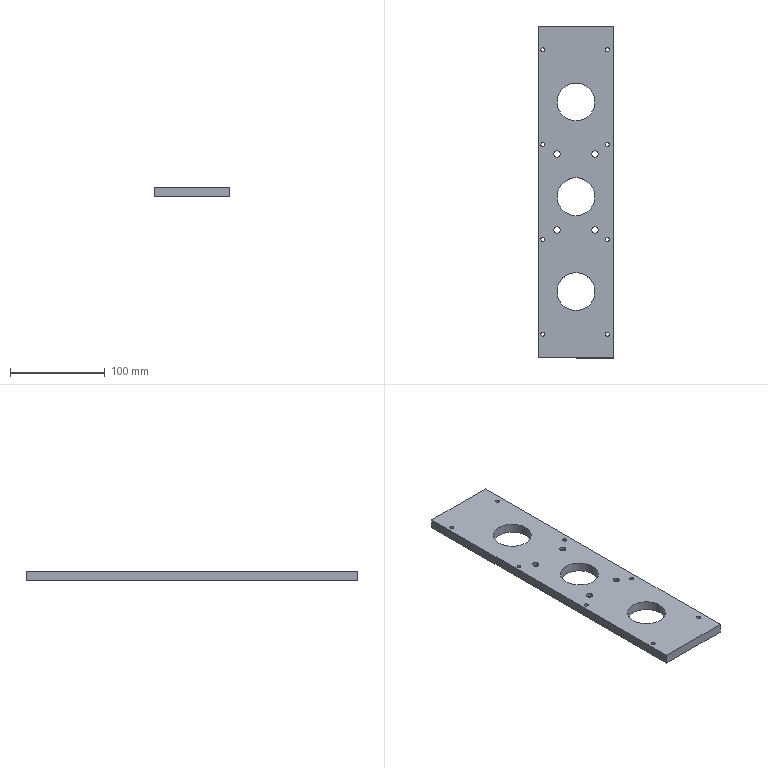Part | SolidWorks | features HoleWzd 2, Extrusion 1, ICE 1, LPattern 1 | 1 solid | 48 faces | box 80 x 350 x 10 mm | volume 238170 mm3 | cylinder 38 | plane 10 | commonest cylinder face diameters 4.2 x16 6.6 x8 11 x8 40 x6
STEP:
#1=CARTESIAN_POINT('',(20.,-5.,10.));
#2=VERTEX_POINT('',#1);
#3=CARTESIAN_POINT('',(-20.,-5.,10.));
#4=VERTEX_POINT('',#3);
#5=CARTESIAN_POINT('',(0.,-5.,10.));
#6=DIRECTION('',(0.,0.,-1.));
#7=DIRECTION('',(1.,0.,0.));
#8=AXIS2_PLACEMENT_3D('',#5,#6,#7);
#9=CIRCLE('',#8,20.);
#10=EDGE_CURVE('',#2,#4,#9,.T.);
#11=ORIENTED_EDGE('',*,*,#10,.F.);
#12=CARTESIAN_POINT('',(20.,-5.,0.));
#13=VERTEX_POINT('',#12);
#14=CARTESIAN_POINT('',(20.,-5.,10.001));
#15=DIRECTION('',(0.,0.,-1.));
#16=VECTOR('',#15,1000.);
#17=LINE('',#14,#16);
#18=EDGE_CURVE('',#2,#13,#17,.T.);
#19=ORIENTED_EDGE('',*,*,#18,.T.);
#20=CARTESIAN_POINT('',(-20.,-5.,0.));
#21=VERTEX_POINT('',#20);
#22=CARTESIAN_POINT('',(0.,-5.,0.));
#23=DIRECTION('',(0.,0.,-1.));
#24=DIRECTION('',(-1.,0.,0.));
#25=AXIS2_PLACEMENT_3D('',#22,#23,#24);
#26=CIRCLE('',#25,20.);
#27=EDGE_CURVE('',#13,#21,#26,.T.);
#28=ORIENTED_EDGE('',*,*,#27,.T.);
#29=CARTESIAN_POINT('',(-20.,-5.,10.001));
#30=DIRECTION('',(0.,0.,-1.));
#31=VECTOR('',#30,1000.);
#32=LINE('',#29,#31);
#33=EDGE_CURVE('',#4,#21,#32,.T.);
#34=ORIENTED_EDGE('',*,*,#33,.F.);
#35=EDGE_LOOP('',(#11,#19,#28,#34));
#36=FACE_OUTER_BOUND('',#35,.T.);
#37=CARTESIAN_POINT('',(0.,-5.,10.001));
#38=DIRECTION('',(0.,0.,-1.));
#39=DIRECTION('',(-1.,0.,0.));
#40=AXIS2_PLACEMENT_3D('',#37,#38,#39);
#41=CYLINDRICAL_SURFACE('',#40,20.);
#42=ADVANCED_FACE('',(#36),#41,.F.);
#43=CARTESIAN_POINT('',(20.,-105.,10.));
#44=VERTEX_POINT('',#43);
#45=CARTESIAN_POINT('',(-20.,-105.,10.));
#46=VERTEX_POINT('',#45);
#47=CARTESIAN_POINT('',(0.,-105.,10.));
#48=DIRECTION('',(0.,0.,-1.));
#49=DIRECTION('',(1.,0.,0.));
#50=AXIS2_PLACEMENT_3D('',#47,#48,#49);
#51=CIRCLE('',#50,20.);
#52=EDGE_CURVE('',#44,#46,#51,.T.);
#53=ORIENTED_EDGE('',*,*,#52,.F.);
#54=CARTESIAN_POINT('',(20.,-105.,0.));
#55=VERTEX_POINT('',#54);
#56=CARTESIAN_POINT('',(20.,-105.,10.001));
#57=DIRECTION('',(0.,0.,-1.));
#58=VECTOR('',#57,1000.);
#59=LINE('',#56,#58);
#60=EDGE_CURVE('',#44,#55,#59,.T.);
#61=ORIENTED_EDGE('',*,*,#60,.T.);
#62=CARTESIAN_POINT('',(-20.,-105.,0.));
#63=VERTEX_POINT('',#62);
#64=CARTESIAN_POINT('',(0.,-105.,0.));
#65=DIRECTION('',(0.,0.,-1.));
#66=DIRECTION('',(-1.,0.,0.));
#67=AXIS2_PLACEMENT_3D('',#64,#65,#66);
#68=CIRCLE('',#67,20.);
#69=EDGE_CURVE('',#55,#63,#68,.T.);
#70=ORIENTED_EDGE('',*,*,#69,.T.);
#71=CARTESIAN_POINT('',(-20.,-105.,10.001));
#72=DIRECTION('',(0.,0.,-1.));
#73=VECTOR('',#72,1000.);
#74=LINE('',#71,#73);
#75=EDGE_CURVE('',#46,#63,#74,.T.);
#76=ORIENTED_EDGE('',*,*,#75,.F.);
#77=EDGE_LOOP('',(#53,#61,#70,#76));
#78=FACE_OUTER_BOUND('',#77,.T.);
#79=CARTESIAN_POINT('',(0.,-105.,10.001));
#80=DIRECTION('',(0.,0.,-1.));
#81=DIRECTION('',(-1.,0.,0.));
#82=AXIS2_PLACEMENT_3D('',#79,#80,#81);
#83=CYLINDRICAL_SURFACE('',#82,20.);
#84=ADVANCED_FACE('',(#78),#83,.F.);
#85=CARTESIAN_POINT('',(25.5,40.,6.8));
#86=VERTEX_POINT('',#85);
#87=CARTESIAN_POINT('',(14.5,40.,6.8));
#88=VERTEX_POINT('',#87);
#89=CARTESIAN_POINT('',(20.,40.,6.8));
#90=DIRECTION('',(0.,0.,-1.));
#91=DIRECTION('',(-1.,0.,0.));
#92=AXIS2_PLACEMENT_3D('',#89,#90,#91);
#93=CIRCLE('',#92,5.5);
#94=EDGE_CURVE('',#86,#88,#93,.T.);
#95=ORIENTED_EDGE('',*,*,#94,.F.);
#96=CARTESIAN_POINT('',(25.5,40.,0.));
#97=VERTEX_POINT('',#96);
#98=CARTESIAN_POINT('',(25.5,40.,0.));
#99=DIRECTION('',(0.,0.,-1.));
#100=VECTOR('',#99,1000.);
#101=LINE('',#98,#100);
#102=EDGE_CURVE('',#86,#97,#101,.T.);
#103=ORIENTED_EDGE('',*,*,#102,.T.);
#104=CARTESIAN_POINT('',(14.5,40.,0.));
#105=VERTEX_POINT('',#104);
#106=CARTESIAN_POINT('',(20.,40.,0.));
#107=DIRECTION('',(0.,0.,-1.));
#108=DIRECTION('',(-1.,0.,0.));
#109=AXIS2_PLACEMENT_3D('',#106,#107,#108);
#110=CIRCLE('',#109,5.5);
#111=EDGE_CURVE('',#97,#105,#110,.T.);
#112=ORIENTED_EDGE('',*,*,#111,.T.);
#113=CARTESIAN_POINT('',(14.5,40.,0.));
#114=DIRECTION('',(0.,0.,-1.));
#115=VECTOR('',#114,1000.);
#116=LINE('',#113,#115);
#117=EDGE_CURVE('',#88,#105,#116,.T.);
#118=ORIENTED_EDGE('',*,*,#117,.F.);
#119=EDGE_LOOP('',(#95,#103,#112,#118));
#120=FACE_OUTER_BOUND('',#119,.T.);
#121=CARTESIAN_POINT('',(20.,40.,0.));
#122=DIRECTION('',(0.,0.,-1.));
#123=DIRECTION('',(-1.,0.,0.));
#124=AXIS2_PLACEMENT_3D('',#121,#122,#123);
#125=CYLINDRICAL_SURFACE('',#124,5.5);
#126=ADVANCED_FACE('',(#120),#125,.F.);
#127=CARTESIAN_POINT('',(16.7,40.,10.));
#128=VERTEX_POINT('',#127);
#129=CARTESIAN_POINT('',(23.3,40.,10.));
#130=VERTEX_POINT('',#129);
#131=CARTESIAN_POINT('',(20.,40.,10.));
#132=DIRECTION('',(0.,0.,1.));
#133=DIRECTION('',(1.,0.,0.));
#134=AXIS2_PLACEMENT_3D('',#131,#132,#133);
#135=CIRCLE('',#134,3.3);
#136=EDGE_CURVE('',#128,#130,#135,.T.);
#137=ORIENTED_EDGE('',*,*,#136,.T.);
#138=CARTESIAN_POINT('',(23.3,40.,6.8));
#139=VERTEX_POINT('',#138);
#140=CARTESIAN_POINT('',(23.3,40.,0.));
#141=DIRECTION('',(0.,0.,-1.));
#142=VECTOR('',#141,1000.);
#143=LINE('',#140,#142);
#144=EDGE_CURVE('',#130,#139,#143,.T.);
#145=ORIENTED_EDGE('',*,*,#144,.T.);
#146=CARTESIAN_POINT('',(16.7,40.,6.8));
#147=VERTEX_POINT('',#146);
#148=CARTESIAN_POINT('',(20.,40.,6.8));
#149=DIRECTION('',(0.,0.,-1.));
#150=DIRECTION('',(-1.,0.,0.));
#151=AXIS2_PLACEMENT_3D('',#148,#149,#150);
#152=CIRCLE('',#151,3.3);
#153=EDGE_CURVE('',#139,#147,#152,.T.);
#154=ORIENTED_EDGE('',*,*,#153,.T.);
#155=CARTESIAN_POINT('',(16.7,40.,0.));
#156=DIRECTION('',(0.,0.,-1.));
#157=VECTOR('',#156,1000.);
#158=LINE('',#155,#157);
#159=EDGE_CURVE('',#128,#147,#158,.T.);
#160=ORIENTED_EDGE('',*,*,#159,.F.);
#161=EDGE_LOOP('',(#137,#145,#154,#160));
#162=FACE_OUTER_BOUND('',#161,.T.);
#163=CARTESIAN_POINT('',(20.,40.,0.));
#164=DIRECTION('',(0.,0.,-1.));
#165=DIRECTION('',(-1.,0.,0.));
#166=AXIS2_PLACEMENT_3D('',#163,#164,#165);
#167=CYLINDRICAL_SURFACE('',#166,3.3);
#168=ADVANCED_FACE('',(#162),#167,.F.);
#169=CARTESIAN_POINT('',(-14.5,40.,6.8));
#170=VERTEX_POINT('',#169);
#171=CARTESIAN_POINT('',(-25.5,40.,6.8));
#172=VERTEX_POINT('',#171);
#173=CARTESIAN_POINT('',(-20.,40.,6.8));
#174=DIRECTION('',(0.,0.,-1.));
#175=DIRECTION('',(-1.,0.,0.));
#176=AXIS2_PLACEMENT_3D('',#173,#174,#175);
#177=CIRCLE('',#176,5.5);
#178=EDGE_CURVE('',#170,#172,#177,.T.);
#179=ORIENTED_EDGE('',*,*,#178,.F.);
#180=CARTESIAN_POINT('',(-14.5,40.,0.));
#181=VERTEX_POINT('',#180);
#182=CARTESIAN_POINT('',(-14.5,40.,0.));
#183=DIRECTION('',(0.,0.,-1.));
#184=VECTOR('',#183,1000.);
#185=LINE('',#182,#184);
#186=EDGE_CURVE('',#170,#181,#185,.T.);
#187=ORIENTED_EDGE('',*,*,#186,.T.);
#188=CARTESIAN_POINT('',(-25.5,40.,0.));
#189=VERTEX_POINT('',#188);
#190=CARTESIAN_POINT('',(-20.,40.,0.));
#191=DIRECTION('',(0.,0.,-1.));
#192=DIRECTION('',(-1.,0.,0.));
#193=AXIS2_PLACEMENT_3D('',#190,#191,#192);
#194=CIRCLE('',#193,5.5);
#195=EDGE_CURVE('',#181,#189,#194,.T.);
#196=ORIENTED_EDGE('',*,*,#195,.T.);
#197=CARTESIAN_POINT('',(-25.5,40.,0.));
#198=DIRECTION('',(0.,0.,-1.));
#199=VECTOR('',#198,1000.);
#200=LINE('',#197,#199);
#201=EDGE_CURVE('',#172,#189,#200,.T.);
#202=ORIENTED_EDGE('',*,*,#201,.F.);
#203=EDGE_LOOP('',(#179,#187,#196,#202));
#204=FACE_OUTER_BOUND('',#203,.T.);
#205=CARTESIAN_POINT('',(-20.,40.,0.));
#206=DIRECTION('',(0.,0.,-1.));
#207=DIRECTION('',(-1.,0.,0.));
#208=AXIS2_PLACEMENT_3D('',#205,#206,#207);
#209=CYLINDRICAL_SURFACE('',#208,5.5);
#210=ADVANCED_FACE('',(#204),#209,.F.);
#211=CARTESIAN_POINT('',(-23.3,40.,10.));
#212=VERTEX_POINT('',#211);
#213=CARTESIAN_POINT('',(-16.7,40.,10.));
#214=VERTEX_POINT('',#213);
#215=CARTESIAN_POINT('',(-20.,40.,10.));
#216=DIRECTION('',(0.,0.,1.));
#217=DIRECTION('',(1.,0.,0.));
#218=AXIS2_PLACEMENT_3D('',#215,#216,#217);
#219=CIRCLE('',#218,3.3);
#220=EDGE_CURVE('',#212,#214,#219,.T.);
#221=ORIENTED_EDGE('',*,*,#220,.T.);
#222=CARTESIAN_POINT('',(-16.7,40.,6.8));
#223=VERTEX_POINT('',#222);
#224=CARTESIAN_POINT('',(-16.7,40.,0.));
#225=DIRECTION('',(0.,0.,-1.));
#226=VECTOR('',#225,1000.);
#227=LINE('',#224,#226);
#228=EDGE_CURVE('',#214,#223,#227,.T.);
#229=ORIENTED_EDGE('',*,*,#228,.T.);
#230=CARTESIAN_POINT('',(-23.3,40.,6.8));
#231=VERTEX_POINT('',#230);
#232=CARTESIAN_POINT('',(-20.,40.,6.8));
#233=DIRECTION('',(0.,0.,-1.));
#234=DIRECTION('',(-1.,0.,0.));
#235=AXIS2_PLACEMENT_3D('',#232,#233,#234);
#236=CIRCLE('',#235,3.3);
#237=EDGE_CURVE('',#223,#231,#236,.T.);
#238=ORIENTED_EDGE('',*,*,#237,.T.);
#239=CARTESIAN_POINT('',(-23.3,40.,0.));
#240=DIRECTION('',(0.,0.,-1.));
#241=VECTOR('',#240,1000.);
#242=LINE('',#239,#241);
#243=EDGE_CURVE('',#212,#231,#242,.T.);
#244=ORIENTED_EDGE('',*,*,#243,.F.);
#245=EDGE_LOOP('',(#221,#229,#238,#244));
#246=FACE_OUTER_BOUND('',#245,.T.);
#247=CARTESIAN_POINT('',(-20.,40.,0.));
#248=DIRECTION('',(0.,0.,-1.));
#249=DIRECTION('',(-1.,0.,0.));
#250=AXIS2_PLACEMENT_3D('',#247,#248,#249);
#251=CYLINDRICAL_SURFACE('',#250,3.3);
#252=ADVANCED_FACE('',(#246),#251,.F.);
#253=CARTESIAN_POINT('',(-14.5,-40.,6.8));
#254=VERTEX_POINT('',#253);
#255=CARTESIAN_POINT('',(-25.5,-40.,6.8));
#256=VERTEX_POINT('',#255);
#257=CARTESIAN_POINT('',(-20.,-40.,6.8));
#258=DIRECTION('',(0.,0.,-1.));
#259=DIRECTION('',(-1.,0.,0.));
#260=AXIS2_PLACEMENT_3D('',#257,#258,#259);
#261=CIRCLE('',#260,5.5);
#262=EDGE_CURVE('',#254,#256,#261,.T.);
#263=ORIENTED_EDGE('',*,*,#262,.F.);
#264=CARTESIAN_POINT('',(-14.5,-40.,0.));
#265=VERTEX_POINT('',#264);
#266=CARTESIAN_POINT('',(-14.5,-40.,0.));
#267=DIRECTION('',(0.,0.,-1.));
#268=VECTOR('',#267,1000.);
#269=LINE('',#266,#268);
#270=EDGE_CURVE('',#254,#265,#269,.T.);
#271=ORIENTED_EDGE('',*,*,#270,.T.);
#272=CARTESIAN_POINT('',(-25.5,-40.,0.));
#273=VERTEX_POINT('',#272);
#274=CARTESIAN_POINT('',(-20.,-40.,0.));
#275=DIRECTION('',(0.,0.,-1.));
#276=DIRECTION('',(-1.,0.,0.));
#277=AXIS2_PLACEMENT_3D('',#274,#275,#276);
#278=CIRCLE('',#277,5.5);
#279=EDGE_CURVE('',#265,#273,#278,.T.);
#280=ORIENTED_EDGE('',*,*,#279,.T.);
#281=CARTESIAN_POINT('',(-25.5,-40.,0.));
#282=DIRECTION('',(0.,0.,-1.));
#283=VECTOR('',#282,1000.);
#284=LINE('',#281,#283);
#285=EDGE_CURVE('',#256,#273,#284,.T.);
#286=ORIENTED_EDGE('',*,*,#285,.F.);
#287=EDGE_LOOP('',(#263,#271,#280,#286));
#288=FACE_OUTER_BOUND('',#287,.T.);
#289=CARTESIAN_POINT('',(-20.,-40.,0.));
#290=DIRECTION('',(0.,0.,-1.));
#291=DIRECTION('',(-1.,0.,0.));
#292=AXIS2_PLACEMENT_3D('',#289,#290,#291);
#293=CYLINDRICAL_SURFACE('',#292,5.5);
#294=ADVANCED_FACE('',(#288),#293,.F.);
#295=CARTESIAN_POINT('',(-23.3,-40.,10.));
#296=VERTEX_POINT('',#295);
#297=CARTESIAN_POINT('',(-16.7,-40.,10.));
#298=VERTEX_POINT('',#297);
#299=CARTESIAN_POINT('',(-20.,-40.,10.));
#300=DIRECTION('',(0.,0.,1.));
#301=DIRECTION('',(1.,0.,0.));
#302=AXIS2_PLACEMENT_3D('',#299,#300,#301);
#303=CIRCLE('',#302,3.3);
#304=EDGE_CURVE('',#296,#298,#303,.T.);
#305=ORIENTED_EDGE('',*,*,#304,.T.);
#306=CARTESIAN_POINT('',(-16.7,-40.,6.8));
#307=VERTEX_POINT('',#306);
#308=CARTESIAN_POINT('',(-16.7,-40.,0.));
#309=DIRECTION('',(0.,0.,-1.));
#310=VECTOR('',#309,1000.);
#311=LINE('',#308,#310);
#312=EDGE_CURVE('',#298,#307,#311,.T.);
#313=ORIENTED_EDGE('',*,*,#312,.T.);
#314=CARTESIAN_POINT('',(-23.3,-40.,6.8));
#315=VERTEX_POINT('',#314);
#316=CARTESIAN_POINT('',(-20.,-40.,6.8));
#317=DIRECTION('',(0.,0.,-1.));
#318=DIRECTION('',(-1.,0.,0.));
#319=AXIS2_PLACEMENT_3D('',#316,#317,#318);
#320=CIRCLE('',#319,3.3);
#321=EDGE_CURVE('',#307,#315,#320,.T.);
#322=ORIENTED_EDGE('',*,*,#321,.T.);
#323=CARTESIAN_POINT('',(-23.3,-40.,0.));
#324=DIRECTION('',(0.,0.,-1.));
#325=VECTOR('',#324,1000.);
#326=LINE('',#323,#325);
#327=EDGE_CURVE('',#296,#315,#326,.T.);
#328=ORIENTED_EDGE('',*,*,#327,.F.);
#329=EDGE_LOOP('',(#305,#313,#322,#328));
#330=FACE_OUTER_BOUND('',#329,.T.);
#331=CARTESIAN_POINT('',(-20.,-40.,0.));
#332=DIRECTION('',(0.,0.,-1.));
#333=DIRECTION('',(-1.,0.,0.));
#334=AXIS2_PLACEMENT_3D('',#331,#332,#333);
#335=CYLINDRICAL_SURFACE('',#334,3.3);
#336=ADVANCED_FACE('',(#330),#335,.F.);
#337=CARTESIAN_POINT('',(25.5,-40.,6.8));
#338=VERTEX_POINT('',#337);
#339=CARTESIAN_POINT('',(14.5,-40.,6.8));
#340=VERTEX_POINT('',#339);
#341=CARTESIAN_POINT('',(20.,-40.,6.8));
#342=DIRECTION('',(0.,0.,-1.));
#343=DIRECTION('',(-1.,0.,0.));
#344=AXIS2_PLACEMENT_3D('',#341,#342,#343);
#345=CIRCLE('',#344,5.5);
#346=EDGE_CURVE('',#338,#340,#345,.T.);
#347=ORIENTED_EDGE('',*,*,#346,.F.);
#348=CARTESIAN_POINT('',(25.5,-40.,0.));
#349=VERTEX_POINT('',#348);
#350=CARTESIAN_POINT('',(25.5,-40.,0.));
#351=DIRECTION('',(0.,0.,-1.));
#352=VECTOR('',#351,1000.);
#353=LINE('',#350,#352);
#354=EDGE_CURVE('',#338,#349,#353,.T.);
#355=ORIENTED_EDGE('',*,*,#354,.T.);
#356=CARTESIAN_POINT('',(14.5,-40.,0.));
#357=VERTEX_POINT('',#356);
#358=CARTESIAN_POINT('',(20.,-40.,0.));
#359=DIRECTION('',(0.,0.,-1.));
#360=DIRECTION('',(-1.,0.,0.));
#361=AXIS2_PLACEMENT_3D('',#358,#359,#360);
#362=CIRCLE('',#361,5.5);
#363=EDGE_CURVE('',#349,#357,#362,.T.);
#364=ORIENTED_EDGE('',*,*,#363,.T.);
#365=CARTESIAN_POINT('',(14.5,-40.,0.));
#366=DIRECTION('',(0.,0.,-1.));
#367=VECTOR('',#366,1000.);
#368=LINE('',#365,#367);
#369=EDGE_CURVE('',#340,#357,#368,.T.);
#370=ORIENTED_EDGE('',*,*,#369,.F.);
#371=EDGE_LOOP('',(#347,#355,#364,#370));
#372=FACE_OUTER_BOUND('',#371,.T.);
#373=CARTESIAN_POINT('',(20.,-40.,0.));
#374=DIRECTION('',(0.,0.,-1.));
#375=DIRECTION('',(-1.,0.,0.));
#376=AXIS2_PLACEMENT_3D('',#373,#374,#375);
#377=CYLINDRICAL_SURFACE('',#376,5.5);
#378=ADVANCED_FACE('',(#372),#377,.F.);
#379=CARTESIAN_POINT('',(16.7,-40.,10.));
#380=VERTEX_POINT('',#379);
#381=CARTESIAN_POINT('',(23.3,-40.,10.));
#382=VERTEX_POINT('',#381);
#383=CARTESIAN_POINT('',(20.,-40.,10.));
#384=DIRECTION('',(0.,0.,1.));
#385=DIRECTION('',(1.,0.,0.));
#386=AXIS2_PLACEMENT_3D('',#383,#384,#385);
#387=CIRCLE('',#386,3.3);
#388=EDGE_CURVE('',#380,#382,#387,.T.);
#389=ORIENTED_EDGE('',*,*,#388,.T.);
#390=CARTESIAN_POINT('',(23.3,-40.,6.8));
#391=VERTEX_POINT('',#390);
#392=CARTESIAN_POINT('',(23.3,-40.,0.));
#393=DIRECTION('',(0.,0.,-1.));
#394=VECTOR('',#393,1000.);
#395=LINE('',#392,#394);
#396=EDGE_CURVE('',#382,#391,#395,.T.);
#397=ORIENTED_EDGE('',*,*,#396,.T.);
#398=CARTESIAN_POINT('',(16.7,-40.,6.8));
#399=VERTEX_POINT('',#398);
#400=CARTESIAN_POINT('',(20.,-40.,6.8));
#401=DIRECTION('',(0.,0.,-1.));
#402=DIRECTION('',(-1.,0.,0.));
#403=AXIS2_PLACEMENT_3D('',#400,#401,#402);
#404=CIRCLE('',#403,3.3);
#405=EDGE_CURVE('',#391,#399,#404,.T.);
#406=ORIENTED_EDGE('',*,*,#405,.T.);
#407=CARTESIAN_POINT('',(16.7,-40.,0.));
#408=DIRECTION('',(0.,0.,-1.));
#409=VECTOR('',#408,1000.);
#410=LINE('',#407,#409);
#411=EDGE_CURVE('',#380,#399,#410,.T.);
#412=ORIENTED_EDGE('',*,*,#411,.F.);
#413=EDGE_LOOP('',(#389,#397,#406,#412));
#414=FACE_OUTER_BOUND('',#413,.T.);
#415=CARTESIAN_POINT('',(20.,-40.,0.));
#416=DIRECTION('',(0.,0.,-1.));
#417=DIRECTION('',(-1.,0.,0.));
#418=AXIS2_PLACEMENT_3D('',#415,#416,#417);
#419=CYLINDRICAL_SURFACE('',#418,3.3);
#420=ADVANCED_FACE('',(#414),#419,.F.);
#421=CARTESIAN_POINT('',(30.9,150.,10.));
#422=VERTEX_POINT('',#421);
#423=CARTESIAN_POINT('',(35.1,150.,10.));
#424=VERTEX_POINT('',#423);
#425=CARTESIAN_POINT('',(33.,150.,10.));
#426=DIRECTION('',(0.,0.,1.));
#427=DIRECTION('',(1.,0.,0.));
#428=AXIS2_PLACEMENT_3D('',#425,#426,#427);
#429=CIRCLE('',#428,2.1);
#430=EDGE_CURVE('',#422,#424,#429,.T.);
#431=ORIENTED_EDGE('',*,*,#430,.T.);
#432=CARTESIAN_POINT('',(35.1,150.,0.));
#433=VERTEX_POINT('',#432);
#434=CARTESIAN_POINT('',(35.1,150.,0.));
#435=DIRECTION('',(0.,0.,-1.));
#436=VECTOR('',#435,1000.);
#437=LINE('',#434,#436);
#438=EDGE_CURVE('',#424,#433,#437,.T.);
#439=ORIENTED_EDGE('',*,*,#438,.T.);
#440=CARTESIAN_POINT('',(30.9,150.,0.));
#441=VERTEX_POINT('',#440);
#442=CARTESIAN_POINT('',(33.,150.,0.));
#443=DIRECTION('',(0.,0.,-1.));
#444=DIRECTION('',(-1.,0.,0.));
#445=AXIS2_PLACEMENT_3D('',#442,#443,#444);
#446=CIRCLE('',#445,2.1);
#447=EDGE_CURVE('',#433,#441,#446,.T.);
#448=ORIENTED_EDGE('',*,*,#447,.T.);
#449=CARTESIAN_POINT('',(30.9,150.,0.));
#450=DIRECTION('',(0.,0.,-1.));
#451=VECTOR('',#450,1000.);
#452=LINE('',#449,#451);
#453=EDGE_CURVE('',#422,#441,#452,.T.);
#454=ORIENTED_EDGE('',*,*,#453,.F.);
#455=EDGE_LOOP('',(#431,#439,#448,#454));
#456=FACE_OUTER_BOUND('',#455,.T.);
#457=CARTESIAN_POINT('',(33.,150.,0.));
#458=DIRECTION('',(0.,0.,-1.));
#459=DIRECTION('',(-1.,0.,0.));
#460=AXIS2_PLACEMENT_3D('',#457,#458,#459);
#461=CYLINDRICAL_SURFACE('',#460,2.1);
#462=ADVANCED_FACE('',(#456),#461,.F.);
#463=CARTESIAN_POINT('',(-37.1,150.,10.));
#464=VERTEX_POINT('',#463);
#465=CARTESIAN_POINT('',(-32.9,150.,10.));
#466=VERTEX_POINT('',#465);
#467=CARTESIAN_POINT('',(-35.,150.,10.));
#468=DIRECTION('',(0.,0.,1.));
#469=DIRECTION('',(1.,0.,0.));
#470=AXIS2_PLACEMENT_3D('',#467,#468,#469);
#471=CIRCLE('',#470,2.1);
#472=EDGE_CURVE('',#464,#466,#471,.T.);
#473=ORIENTED_EDGE('',*,*,#472,.T.);
#474=CARTESIAN_POINT('',(-32.9,150.,0.));
#475=VERTEX_POINT('',#474);
#476=CARTESIAN_POINT('',(-32.9,150.,0.));
#477=DIRECTION('',(0.,0.,-1.));
#478=VECTOR('',#477,1000.);
#479=LINE('',#476,#478);
#480=EDGE_CURVE('',#466,#475,#479,.T.);
#481=ORIENTED_EDGE('',*,*,#480,.T.);
#482=CARTESIAN_POINT('',(-37.1,150.,0.));
#483=VERTEX_POINT('',#482);
#484=CARTESIAN_POINT('',(-35.,150.,0.));
#485=DIRECTION('',(0.,0.,-1.));
#486=DIRECTION('',(-1.,0.,0.));
#487=AXIS2_PLACEMENT_3D('',#484,#485,#486);
#488=CIRCLE('',#487,2.1);
#489=EDGE_CURVE('',#475,#483,#488,.T.);
#490=ORIENTED_EDGE('',*,*,#489,.T.);
#491=CARTESIAN_POINT('',(-37.1,150.,0.));
#492=DIRECTION('',(0.,0.,-1.));
#493=VECTOR('',#492,1000.);
#494=LINE('',#491,#493);
#495=EDGE_CURVE('',#464,#483,#494,.T.);
#496=ORIENTED_EDGE('',*,*,#495,.F.);
#497=EDGE_LOOP('',(#473,#481,#490,#496));
#498=FACE_OUTER_BOUND('',#497,.T.);
#499=CARTESIAN_POINT('',(-35.,150.,0.));
#500=DIRECTION('',(0.,0.,-1.));
#501=DIRECTION('',(-1.,0.,0.));
#502=AXIS2_PLACEMENT_3D('',#499,#500,#501);
#503=CYLINDRICAL_SURFACE('',#502,2.1);
#504=ADVANCED_FACE('',(#498),#503,.F.);
#505=CARTESIAN_POINT('',(30.9,50.,10.));
#506=VERTEX_POINT('',#505);
#507=CARTESIAN_POINT('',(35.1,50.,10.));
#508=VERTEX_POINT('',#507);
#509=CARTESIAN_POINT('',(33.,50.,10.));
#510=DIRECTION('',(0.,0.,1.));
#511=DIRECTION('',(1.,0.,0.));
#512=AXIS2_PLACEMENT_3D('',#509,#510,#511);
#513=CIRCLE('',#512,2.1);
#514=EDGE_CURVE('',#506,#508,#513,.T.);
#515=ORIENTED_EDGE('',*,*,#514,.T.);
#516=CARTESIAN_POINT('',(35.1,50.,0.));
#517=VERTEX_POINT('',#516);
#518=CARTESIAN_POINT('',(35.1,50.,0.));
#519=DIRECTION('',(0.,0.,-1.));
#520=VECTOR('',#519,1000.);
#521=LINE('',#518,#520);
#522=EDGE_CURVE('',#508,#517,#521,.T.);
#523=ORIENTED_EDGE('',*,*,#522,.T.);
#524=CARTESIAN_POINT('',(30.9,50.,0.));
#525=VERTEX_POINT('',#524);
#526=CARTESIAN_POINT('',(33.,50.,0.));
#527=DIRECTION('',(0.,0.,-1.));
#528=DIRECTION('',(-1.,0.,0.));
#529=AXIS2_PLACEMENT_3D('',#526,#527,#528);
#530=CIRCLE('',#529,2.1);
#531=EDGE_CURVE('',#517,#525,#530,.T.);
#532=ORIENTED_EDGE('',*,*,#531,.T.);
#533=CARTESIAN_POINT('',(30.9,50.,0.));
#534=DIRECTION('',(0.,0.,-1.));
#535=VECTOR('',#534,1000.);
#536=LINE('',#533,#535);
#537=EDGE_CURVE('',#506,#525,#536,.T.);
#538=ORIENTED_EDGE('',*,*,#537,.F.);
#539=EDGE_LOOP('',(#515,#523,#532,#538));
#540=FACE_OUTER_BOUND('',#539,.T.);
#541=CARTESIAN_POINT('',(33.,50.,0.));
#542=DIRECTION('',(0.,0.,-1.));
#543=DIRECTION('',(-1.,0.,0.));
#544=AXIS2_PLACEMENT_3D('',#541,#542,#543);
#545=CYLINDRICAL_SURFACE('',#544,2.1);
#546=ADVANCED_FACE('',(#540),#545,.F.);
#547=CARTESIAN_POINT('',(-37.1,50.,10.));
#548=VERTEX_POINT('',#547);
#549=CARTESIAN_POINT('',(-32.9,50.,10.));
#550=VERTEX_POINT('',#549);
#551=CARTESIAN_POINT('',(-35.,50.,10.));
#552=DIRECTION('',(0.,0.,1.));
#553=DIRECTION('',(1.,0.,0.));
#554=AXIS2_PLACEMENT_3D('',#551,#552,#553);
#555=CIRCLE('',#554,2.1);
#556=EDGE_CURVE('',#548,#550,#555,.T.);
#557=ORIENTED_EDGE('',*,*,#556,.T.);
#558=CARTESIAN_POINT('',(-32.9,50.,0.));
#559=VERTEX_POINT('',#558);
#560=CARTESIAN_POINT('',(-32.9,50.,0.));
#561=DIRECTION('',(0.,0.,-1.));
#562=VECTOR('',#561,1000.);
#563=LINE('',#560,#562);
#564=EDGE_CURVE('',#550,#559,#563,.T.);
#565=ORIENTED_EDGE('',*,*,#564,.T.);
#566=CARTESIAN_POINT('',(-37.1,50.,0.));
#567=VERTEX_POINT('',#566);
#568=CARTESIAN_POINT('',(-35.,50.,0.));
#569=DIRECTION('',(0.,0.,-1.));
#570=DIRECTION('',(-1.,0.,0.));
#571=AXIS2_PLACEMENT_3D('',#568,#569,#570);
#572=CIRCLE('',#571,2.1);
#573=EDGE_CURVE('',#559,#567,#572,.T.);
#574=ORIENTED_EDGE('',*,*,#573,.T.);
#575=CARTESIAN_POINT('',(-37.1,50.,0.));
#576=DIRECTION('',(0.,0.,-1.));
#577=VECTOR('',#576,1000.);
#578=LINE('',#575,#577);
#579=EDGE_CURVE('',#548,#567,#578,.T.);
#580=ORIENTED_EDGE('',*,*,#579,.F.);
#581=EDGE_LOOP('',(#557,#565,#574,#580));
#582=FACE_OUTER_BOUND('',#581,.T.);
#583=CARTESIAN_POINT('',(-35.,50.,0.));
#584=DIRECTION('',(0.,0.,-1.));
#585=DIRECTION('',(-1.,0.,0.));
#586=AXIS2_PLACEMENT_3D('',#583,#584,#585);
#587=CYLINDRICAL_SURFACE('',#586,2.1);
#588=ADVANCED_FACE('',(#582),#587,.F.);
#589=CARTESIAN_POINT('',(30.9,-50.,10.));
#590=VERTEX_POINT('',#589);
#591=CARTESIAN_POINT('',(35.1,-50.,10.));
#592=VERTEX_POINT('',#591);
#593=CARTESIAN_POINT('',(33.,-50.,10.));
#594=DIRECTION('',(0.,0.,1.));
#595=DIRECTION('',(1.,0.,0.));
#596=AXIS2_PLACEMENT_3D('',#593,#594,#595);
#597=CIRCLE('',#596,2.1);
#598=EDGE_CURVE('',#590,#592,#597,.T.);
#599=ORIENTED_EDGE('',*,*,#598,.T.);
#600=CARTESIAN_POINT('',(35.1,-50.,0.));
#601=VERTEX_POINT('',#600);
#602=CARTESIAN_POINT('',(35.1,-50.,0.));
#603=DIRECTION('',(0.,0.,-1.));
#604=VECTOR('',#603,1000.);
#605=LINE('',#602,#604);
#606=EDGE_CURVE('',#592,#601,#605,.T.);
#607=ORIENTED_EDGE('',*,*,#606,.T.);
#608=CARTESIAN_POINT('',(30.9,-50.,0.));
#609=VERTEX_POINT('',#608);
#610=CARTESIAN_POINT('',(33.,-50.,0.));
#611=DIRECTION('',(0.,0.,-1.));
#612=DIRECTION('',(-1.,0.,0.));
#613=AXIS2_PLACEMENT_3D('',#610,#611,#612);
#614=CIRCLE('',#613,2.1);
#615=EDGE_CURVE('',#601,#609,#614,.T.);
#616=ORIENTED_EDGE('',*,*,#615,.T.);
#617=CARTESIAN_POINT('',(30.9,-50.,0.));
#618=DIRECTION('',(0.,0.,-1.));
#619=VECTOR('',#618,1000.);
#620=LINE('',#617,#619);
#621=EDGE_CURVE('',#590,#609,#620,.T.);
#622=ORIENTED_EDGE('',*,*,#621,.F.);
#623=EDGE_LOOP('',(#599,#607,#616,#622));
#624=FACE_OUTER_BOUND('',#623,.T.);
#625=CARTESIAN_POINT('',(33.,-50.,0.));
#626=DIRECTION('',(0.,0.,-1.));
#627=DIRECTION('',(-1.,0.,0.));
#628=AXIS2_PLACEMENT_3D('',#625,#626,#627);
#629=CYLINDRICAL_SURFACE('',#628,2.1);
#630=ADVANCED_FACE('',(#624),#629,.F.);
#631=CARTESIAN_POINT('',(-37.1,-50.,10.));
#632=VERTEX_POINT('',#631);
#633=CARTESIAN_POINT('',(-32.9,-50.,10.));
#634=VERTEX_POINT('',#633);
#635=CARTESIAN_POINT('',(-35.,-50.,10.));
#636=DIRECTION('',(0.,0.,1.));
#637=DIRECTION('',(1.,0.,0.));
#638=AXIS2_PLACEMENT_3D('',#635,#636,#637);
#639=CIRCLE('',#638,2.1);
#640=EDGE_CURVE('',#632,#634,#639,.T.);
#641=ORIENTED_EDGE('',*,*,#640,.T.);
#642=CARTESIAN_POINT('',(-32.9,-50.,0.));
#643=VERTEX_POINT('',#642);
#644=CARTESIAN_POINT('',(-32.9,-50.,0.));
#645=DIRECTION('',(0.,0.,-1.));
#646=VECTOR('',#645,1000.);
#647=LINE('',#644,#646);
#648=EDGE_CURVE('',#634,#643,#647,.T.);
#649=ORIENTED_EDGE('',*,*,#648,.T.);
#650=CARTESIAN_POINT('',(-37.1,-50.,0.));
#651=VERTEX_POINT('',#650);
#652=CARTESIAN_POINT('',(-35.,-50.,0.));
#653=DIRECTION('',(0.,0.,-1.));
#654=DIRECTION('',(-1.,0.,0.));
#655=AXIS2_PLACEMENT_3D('',#652,#653,#654);
#656=CIRCLE('',#655,2.1);
#657=EDGE_CURVE('',#643,#651,#656,.T.);
#658=ORIENTED_EDGE('',*,*,#657,.T.);
#659=CARTESIAN_POINT('',(-37.1,-50.,0.));
#660=DIRECTION('',(0.,0.,-1.));
#661=VECTOR('',#660,1000.);
#662=LINE('',#659,#661);
#663=EDGE_CURVE('',#632,#651,#662,.T.);
#664=ORIENTED_EDGE('',*,*,#663,.F.);
#665=EDGE_LOOP('',(#641,#649,#658,#664));
#666=FACE_OUTER_BOUND('',#665,.T.);
#667=CARTESIAN_POINT('',(-35.,-50.,0.));
#668=DIRECTION('',(0.,0.,-1.));
#669=DIRECTION('',(-1.,0.,0.));
#670=AXIS2_PLACEMENT_3D('',#667,#668,#669);
#671=CYLINDRICAL_SURFACE('',#670,2.1);
#672=ADVANCED_FACE('',(#666),#671,.F.);
#673=CARTESIAN_POINT('',(30.9,-150.,10.));
#674=VERTEX_POINT('',#673);
#675=CARTESIAN_POINT('',(35.1,-150.,10.));
#676=VERTEX_POINT('',#675);
#677=CARTESIAN_POINT('',(33.,-150.,10.));
#678=DIRECTION('',(0.,0.,1.));
#679=DIRECTION('',(1.,0.,0.));
#680=AXIS2_PLACEMENT_3D('',#677,#678,#679);
#681=CIRCLE('',#680,2.1);
#682=EDGE_CURVE('',#674,#676,#681,.T.);
#683=ORIENTED_EDGE('',*,*,#682,.T.);
#684=CARTESIAN_POINT('',(35.1,-150.,0.));
#685=VERTEX_POINT('',#684);
#686=CARTESIAN_POINT('',(35.1,-150.,0.));
#687=DIRECTION('',(0.,0.,-1.));
#688=VECTOR('',#687,1000.);
#689=LINE('',#686,#688);
#690=EDGE_CURVE('',#676,#685,#689,.T.);
#691=ORIENTED_EDGE('',*,*,#690,.T.);
#692=CARTESIAN_POINT('',(30.9,-150.,0.));
#693=VERTEX_POINT('',#692);
#694=CARTESIAN_POINT('',(33.,-150.,0.));
#695=DIRECTION('',(0.,0.,-1.));
#696=DIRECTION('',(-1.,0.,0.));
#697=AXIS2_PLACEMENT_3D('',#694,#695,#696);
#698=CIRCLE('',#697,2.1);
#699=EDGE_CURVE('',#685,#693,#698,.T.);
#700=ORIENTED_EDGE('',*,*,#699,.T.);
#701=CARTESIAN_POINT('',(30.9,-150.,0.));
#702=DIRECTION('',(0.,0.,-1.));
#703=VECTOR('',#702,1000.);
#704=LINE('',#701,#703);
#705=EDGE_CURVE('',#674,#693,#704,.T.);
#706=ORIENTED_EDGE('',*,*,#705,.F.);
#707=EDGE_LOOP('',(#683,#691,#700,#706));
#708=FACE_OUTER_BOUND('',#707,.T.);
#709=CARTESIAN_POINT('',(33.,-150.,0.));
#710=DIRECTION('',(0.,0.,-1.));
#711=DIRECTION('',(-1.,0.,0.));
#712=AXIS2_PLACEMENT_3D('',#709,#710,#711);
#713=CYLINDRICAL_SURFACE('',#712,2.1);
#714=ADVANCED_FACE('',(#708),#713,.F.);
#715=CARTESIAN_POINT('',(-37.1,-150.,10.));
#716=VERTEX_POINT('',#715);
#717=CARTESIAN_POINT('',(-32.9,-150.,10.));
#718=VERTEX_POINT('',#717);
#719=CARTESIAN_POINT('',(-35.,-150.,10.));
#720=DIRECTION('',(0.,0.,1.));
#721=DIRECTION('',(1.,0.,0.));
#722=AXIS2_PLACEMENT_3D('',#719,#720,#721);
#723=CIRCLE('',#722,2.1);
#724=EDGE_CURVE('',#716,#718,#723,.T.);
#725=ORIENTED_EDGE('',*,*,#724,.T.);
#726=CARTESIAN_POINT('',(-32.9,-150.,0.));
#727=VERTEX_POINT('',#726);
#728=CARTESIAN_POINT('',(-32.9,-150.,0.));
#729=DIRECTION('',(0.,0.,-1.));
#730=VECTOR('',#729,1000.);
#731=LINE('',#728,#730);
#732=EDGE_CURVE('',#718,#727,#731,.T.);
#733=ORIENTED_EDGE('',*,*,#732,.T.);
#734=CARTESIAN_POINT('',(-37.1,-150.,0.));
#735=VERTEX_POINT('',#734);
#736=CARTESIAN_POINT('',(-35.,-150.,0.));
#737=DIRECTION('',(0.,0.,-1.));
#738=DIRECTION('',(-1.,0.,0.));
#739=AXIS2_PLACEMENT_3D('',#736,#737,#738);
#740=CIRCLE('',#739,2.1);
#741=EDGE_CURVE('',#727,#735,#740,.T.);
#742=ORIENTED_EDGE('',*,*,#741,.T.);
#743=CARTESIAN_POINT('',(-37.1,-150.,0.));
#744=DIRECTION('',(0.,0.,-1.));
#745=VECTOR('',#744,1000.);
#746=LINE('',#743,#745);
#747=EDGE_CURVE('',#716,#735,#746,.T.);
#748=ORIENTED_EDGE('',*,*,#747,.F.);
#749=EDGE_LOOP('',(#725,#733,#742,#748));
#750=FACE_OUTER_BOUND('',#749,.T.);
#751=CARTESIAN_POINT('',(-35.,-150.,0.));
#752=DIRECTION('',(0.,0.,-1.));
#753=DIRECTION('',(-1.,0.,0.));
#754=AXIS2_PLACEMENT_3D('',#751,#752,#753);
#755=CYLINDRICAL_SURFACE('',#754,2.1);
#756=ADVANCED_FACE('',(#750),#755,.F.);
#757=CARTESIAN_POINT('',(20.,95.,10.));
#758=VERTEX_POINT('',#757);
#759=CARTESIAN_POINT('',(-20.,95.,10.));
#760=VERTEX_POINT('',#759);
#761=CARTESIAN_POINT('',(0.,95.,10.));
#762=DIRECTION('',(0.,0.,-1.));
#763=DIRECTION('',(1.,0.,0.));
#764=AXIS2_PLACEMENT_3D('',#761,#762,#763);
#765=CIRCLE('',#764,20.);
#766=EDGE_CURVE('',#758,#760,#765,.T.);
#767=ORIENTED_EDGE('',*,*,#766,.F.);
#768=CARTESIAN_POINT('',(20.,95.,0.));
#769=VERTEX_POINT('',#768);
#770=CARTESIAN_POINT('',(20.,95.,10.001));
#771=DIRECTION('',(0.,0.,-1.));
#772=VECTOR('',#771,1000.);
#773=LINE('',#770,#772);
#774=EDGE_CURVE('',#758,#769,#773,.T.);
#775=ORIENTED_EDGE('',*,*,#774,.T.);
#776=CARTESIAN_POINT('',(-20.,95.,0.));
#777=VERTEX_POINT('',#776);
#778=CARTESIAN_POINT('',(0.,95.,0.));
#779=DIRECTION('',(0.,0.,-1.));
#780=DIRECTION('',(-1.,0.,0.));
#781=AXIS2_PLACEMENT_3D('',#778,#779,#780);
#782=CIRCLE('',#781,20.);
#783=EDGE_CURVE('',#769,#777,#782,.T.);
#784=ORIENTED_EDGE('',*,*,#783,.T.);
#785=CARTESIAN_POINT('',(-20.,95.,10.001));
#786=DIRECTION('',(0.,0.,-1.));
#787=VECTOR('',#786,1000.);
#788=LINE('',#785,#787);
#789=EDGE_CURVE('',#760,#777,#788,.T.);
#790=ORIENTED_EDGE('',*,*,#789,.F.);
#791=EDGE_LOOP('',(#767,#775,#784,#790));
#792=FACE_OUTER_BOUND('',#791,.T.);
#793=CARTESIAN_POINT('',(0.,95.,10.001));
#794=DIRECTION('',(0.,0.,-1.));
#795=DIRECTION('',(-1.,0.,0.));
#796=AXIS2_PLACEMENT_3D('',#793,#794,#795);
#797=CYLINDRICAL_SURFACE('',#796,20.);
#798=ADVANCED_FACE('',(#792),#797,.F.);
#799=ORIENTED_EDGE('',*,*,#774,.F.);
#800=CARTESIAN_POINT('',(0.,95.,10.));
#801=DIRECTION('',(0.,0.,-1.));
#802=DIRECTION('',(1.,0.,0.));
#803=AXIS2_PLACEMENT_3D('',#800,#801,#802);
#804=CIRCLE('',#803,20.);
#805=EDGE_CURVE('',#760,#758,#804,.T.);
#806=ORIENTED_EDGE('',*,*,#805,.F.);
#807=ORIENTED_EDGE('',*,*,#789,.T.);
#808=CARTESIAN_POINT('',(0.,95.,0.));
#809=DIRECTION('',(0.,0.,-1.));
#810=DIRECTION('',(-1.,0.,0.));
#811=AXIS2_PLACEMENT_3D('',#808,#809,#810);
#812=CIRCLE('',#811,20.);
#813=EDGE_CURVE('',#777,#769,#812,.T.);
#814=ORIENTED_EDGE('',*,*,#813,.T.);
#815=EDGE_LOOP('',(#799,#806,#807,#814));
#816=FACE_OUTER_BOUND('',#815,.T.);
#817=CARTESIAN_POINT('',(0.,95.,10.001));
#818=DIRECTION('',(0.,0.,-1.));
#819=DIRECTION('',(-1.,0.,0.));
#820=AXIS2_PLACEMENT_3D('',#817,#818,#819);
#821=CYLINDRICAL_SURFACE('',#820,20.);
#822=ADVANCED_FACE('',(#816),#821,.F.);
#823=CARTESIAN_POINT('',(0.,-5.,0.));
#824=DIRECTION('',(0.,0.,-1.));
#825=DIRECTION('',(-1.,0.,0.));
#826=AXIS2_PLACEMENT_3D('',#823,#824,#825);
#827=CIRCLE('',#826,20.);
#828=EDGE_CURVE('',#21,#13,#827,.T.);
#829=ORIENTED_EDGE('',*,*,#828,.F.);
#830=ORIENTED_EDGE('',*,*,#27,.F.);
#831=EDGE_LOOP('',(#829,#830));
#832=FACE_BOUND('',#831,.T.);
#833=CARTESIAN_POINT('',(0.,-105.,0.));
#834=DIRECTION('',(0.,0.,-1.));
#835=DIRECTION('',(-1.,0.,0.));
#836=AXIS2_PLACEMENT_3D('',#833,#834,#835);
#837=CIRCLE('',#836,20.);
#838=EDGE_CURVE('',#63,#55,#837,.T.);
#839=ORIENTED_EDGE('',*,*,#838,.F.);
#840=ORIENTED_EDGE('',*,*,#69,.F.);
#841=EDGE_LOOP('',(#839,#840));
#842=FACE_BOUND('',#841,.T.);
#843=CARTESIAN_POINT('',(-20.,-40.,0.));
#844=DIRECTION('',(0.,0.,-1.));
#845=DIRECTION('',(-1.,0.,0.));
#846=AXIS2_PLACEMENT_3D('',#843,#844,#845);
#847=CIRCLE('',#846,5.5);
#848=EDGE_CURVE('',#273,#265,#847,.T.);
#849=ORIENTED_EDGE('',*,*,#848,.F.);
#850=ORIENTED_EDGE('',*,*,#279,.F.);
#851=EDGE_LOOP('',(#849,#850));
#852=FACE_BOUND('',#851,.T.);
#853=CARTESIAN_POINT('',(20.,-40.,0.));
#854=DIRECTION('',(0.,0.,-1.));
#855=DIRECTION('',(-1.,0.,0.));
#856=AXIS2_PLACEMENT_3D('',#853,#854,#855);
#857=CIRCLE('',#856,5.5);
#858=EDGE_CURVE('',#357,#349,#857,.T.);
#859=ORIENTED_EDGE('',*,*,#858,.F.);
#860=ORIENTED_EDGE('',*,*,#363,.F.);
#861=EDGE_LOOP('',(#859,#860));
#862=FACE_BOUND('',#861,.T.);
#863=CARTESIAN_POINT('',(33.,150.,0.));
#864=DIRECTION('',(0.,0.,-1.));
#865=DIRECTION('',(-1.,0.,0.));
#866=AXIS2_PLACEMENT_3D('',#863,#864,#865);
#867=CIRCLE('',#866,2.1);
#868=EDGE_CURVE('',#441,#433,#867,.T.);
#869=ORIENTED_EDGE('',*,*,#868,.F.);
#870=ORIENTED_EDGE('',*,*,#447,.F.);
#871=EDGE_LOOP('',(#869,#870));
#872=FACE_BOUND('',#871,.T.);
#873=CARTESIAN_POINT('',(-35.,150.,0.));
#874=DIRECTION('',(0.,0.,-1.));
#875=DIRECTION('',(-1.,0.,0.));
#876=AXIS2_PLACEMENT_3D('',#873,#874,#875);
#877=CIRCLE('',#876,2.1);
#878=EDGE_CURVE('',#483,#475,#877,.T.);
#879=ORIENTED_EDGE('',*,*,#878,.F.);
#880=ORIENTED_EDGE('',*,*,#489,.F.);
#881=EDGE_LOOP('',(#879,#880));
#882=FACE_BOUND('',#881,.T.);
#883=CARTESIAN_POINT('',(-35.,-150.,0.));
#884=DIRECTION('',(0.,0.,-1.));
#885=DIRECTION('',(-1.,0.,0.));
#886=AXIS2_PLACEMENT_3D('',#883,#884,#885);
#887=CIRCLE('',#886,2.1);
#888=EDGE_CURVE('',#735,#727,#887,.T.);
#889=ORIENTED_EDGE('',*,*,#888,.F.);
#890=ORIENTED_EDGE('',*,*,#741,.F.);
#891=EDGE_LOOP('',(#889,#890));
#892=FACE_BOUND('',#891,.T.);
#893=CARTESIAN_POINT('',(-40.,175.,0.));
#894=VERTEX_POINT('',#893);
#895=CARTESIAN_POINT('',(-40.,-175.,0.));
#896=VERTEX_POINT('',#895);
#897=CARTESIAN_POINT('',(-40.,-175.,0.));
#898=DIRECTION('',(0.,-1.,0.));
#899=VECTOR('',#898,1000.);
#900=LINE('',#897,#899);
#901=EDGE_CURVE('',#894,#896,#900,.T.);
#902=ORIENTED_EDGE('',*,*,#901,.F.);
#903=CARTESIAN_POINT('',(40.,175.,0.));
#904=VERTEX_POINT('',#903);
#905=CARTESIAN_POINT('',(40.,175.,0.));
#906=DIRECTION('',(-1.,0.,0.));
#907=VECTOR('',#906,1000.);
#908=LINE('',#905,#907);
#909=EDGE_CURVE('',#904,#894,#908,.T.);
#910=ORIENTED_EDGE('',*,*,#909,.F.);
#911=CARTESIAN_POINT('',(40.,-175.,0.));
#912=VERTEX_POINT('',#911);
#913=CARTESIAN_POINT('',(40.,-175.,0.));
#914=DIRECTION('',(0.,1.,0.));
#915=VECTOR('',#914,1000.);
#916=LINE('',#913,#915);
#917=EDGE_CURVE('',#912,#904,#916,.T.);
#918=ORIENTED_EDGE('',*,*,#917,.F.);
#919=CARTESIAN_POINT('',(40.,-175.,0.));
#920=DIRECTION('',(1.,0.,0.));
#921=VECTOR('',#920,1000.);
#922=LINE('',#919,#921);
#923=EDGE_CURVE('',#896,#912,#922,.T.);
#924=ORIENTED_EDGE('',*,*,#923,.F.);
#925=EDGE_LOOP('',(#902,#910,#918,#924));
#926=FACE_OUTER_BOUND('',#925,.T.);
#927=CARTESIAN_POINT('',(33.,-150.,0.));
#928=DIRECTION('',(0.,0.,-1.));
#929=DIRECTION('',(-1.,0.,0.));
#930=AXIS2_PLACEMENT_3D('',#927,#928,#929);
#931=CIRCLE('',#930,2.1);
#932=EDGE_CURVE('',#693,#685,#931,.T.);
#933=ORIENTED_EDGE('',*,*,#932,.F.);
#934=ORIENTED_EDGE('',*,*,#699,.F.);
#935=EDGE_LOOP('',(#933,#934));
#936=FACE_BOUND('',#935,.T.);
#937=CARTESIAN_POINT('',(-35.,-50.,0.));
#938=DIRECTION('',(0.,0.,-1.));
#939=DIRECTION('',(-1.,0.,0.));
#940=AXIS2_PLACEMENT_3D('',#937,#938,#939);
#941=CIRCLE('',#940,2.1);
#942=EDGE_CURVE('',#651,#643,#941,.T.);
#943=ORIENTED_EDGE('',*,*,#942,.F.);
#944=ORIENTED_EDGE('',*,*,#657,.F.);
#945=EDGE_LOOP('',(#943,#944));
#946=FACE_BOUND('',#945,.T.);
#947=CARTESIAN_POINT('',(33.,-50.,0.));
#948=DIRECTION('',(0.,0.,-1.));
#949=DIRECTION('',(-1.,0.,0.));
#950=AXIS2_PLACEMENT_3D('',#947,#948,#949);
#951=CIRCLE('',#950,2.1);
#952=EDGE_CURVE('',#609,#601,#951,.T.);
#953=ORIENTED_EDGE('',*,*,#952,.F.);
#954=ORIENTED_EDGE('',*,*,#615,.F.);
#955=EDGE_LOOP('',(#953,#954));
#956=FACE_BOUND('',#955,.T.);
#957=CARTESIAN_POINT('',(-35.,50.,0.));
#958=DIRECTION('',(0.,0.,-1.));
#959=DIRECTION('',(-1.,0.,0.));
#960=AXIS2_PLACEMENT_3D('',#957,#958,#959);
#961=CIRCLE('',#960,2.1);
#962=EDGE_CURVE('',#567,#559,#961,.T.);
#963=ORIENTED_EDGE('',*,*,#962,.F.);
#964=ORIENTED_EDGE('',*,*,#573,.F.);
#965=EDGE_LOOP('',(#963,#964));
#966=FACE_BOUND('',#965,.T.);
#967=CARTESIAN_POINT('',(33.,50.,0.));
#968=DIRECTION('',(0.,0.,-1.));
#969=DIRECTION('',(-1.,0.,0.));
#970=AXIS2_PLACEMENT_3D('',#967,#968,#969);
#971=CIRCLE('',#970,2.1);
#972=EDGE_CURVE('',#525,#517,#971,.T.);
#973=ORIENTED_EDGE('',*,*,#972,.F.);
#974=ORIENTED_EDGE('',*,*,#531,.F.);
#975=EDGE_LOOP('',(#973,#974));
#976=FACE_BOUND('',#975,.T.);
#977=CARTESIAN_POINT('',(-20.,40.,0.));
#978=DIRECTION('',(0.,0.,-1.));
#979=DIRECTION('',(-1.,0.,0.));
#980=AXIS2_PLACEMENT_3D('',#977,#978,#979);
#981=CIRCLE('',#980,5.5);
#982=EDGE_CURVE('',#189,#181,#981,.T.);
#983=ORIENTED_EDGE('',*,*,#982,.F.);
#984=ORIENTED_EDGE('',*,*,#195,.F.);
#985=EDGE_LOOP('',(#983,#984));
#986=FACE_BOUND('',#985,.T.);
#987=CARTESIAN_POINT('',(20.,40.,0.));
#988=DIRECTION('',(0.,0.,-1.));
#989=DIRECTION('',(-1.,0.,0.));
#990=AXIS2_PLACEMENT_3D('',#987,#988,#989);
#991=CIRCLE('',#990,5.5);
#992=EDGE_CURVE('',#105,#97,#991,.T.);
#993=ORIENTED_EDGE('',*,*,#992,.F.);
#994=ORIENTED_EDGE('',*,*,#111,.F.);
#995=EDGE_LOOP('',(#993,#994));
#996=FACE_BOUND('',#995,.T.);
#997=ORIENTED_EDGE('',*,*,#813,.F.);
#998=ORIENTED_EDGE('',*,*,#783,.F.);
#999=EDGE_LOOP('',(#997,#998));
#1000=FACE_BOUND('',#999,.T.);
#1001=CARTESIAN_POINT('',(0.,0.,0.));
#1002=DIRECTION('',(0.,0.,1.));
#1003=DIRECTION('',(1.,0.,0.));
#1004=AXIS2_PLACEMENT_3D('',#1001,#1002,#1003);
#1005=PLANE('',#1004);
#1006=ADVANCED_FACE('',(#832,#842,#852,#862,#872,#882,#892,#926,#936,#946,#956,#966,#976,#986,#996,#1000),#1005,.F.);
#1007=ORIENTED_EDGE('',*,*,#901,.T.);
#1008=CARTESIAN_POINT('',(-40.,-175.,10.));
#1009=VERTEX_POINT('',#1008);
#1010=CARTESIAN_POINT('',(-40.,-175.,10.));
#1011=DIRECTION('',(0.,0.,-1.));
#1012=VECTOR('',#1011,1000.);
#1013=LINE('',#1010,#1012);
#1014=EDGE_CURVE('',#1009,#896,#1013,.T.);
#1015=ORIENTED_EDGE('',*,*,#1014,.F.);
#1016=CARTESIAN_POINT('',(-40.,175.,10.));
#1017=VERTEX_POINT('',#1016);
#1018=CARTESIAN_POINT('',(-40.,-175.,10.));
#1019=DIRECTION('',(0.,-1.,0.));
#1020=VECTOR('',#1019,1000.);
#1021=LINE('',#1018,#1020);
#1022=EDGE_CURVE('',#1017,#1009,#1021,.T.);
#1023=ORIENTED_EDGE('',*,*,#1022,.F.);
#1024=CARTESIAN_POINT('',(-40.,175.,10.));
#1025=DIRECTION('',(0.,0.,-1.));
#1026=VECTOR('',#1025,1000.);
#1027=LINE('',#1024,#1026);
#1028=EDGE_CURVE('',#1017,#894,#1027,.T.);
#1029=ORIENTED_EDGE('',*,*,#1028,.T.);
#1030=EDGE_LOOP('',(#1007,#1015,#1023,#1029));
#1031=FACE_OUTER_BOUND('',#1030,.T.);
#1032=CARTESIAN_POINT('',(-40.,-175.,10.));
#1033=DIRECTION('',(1.,0.,0.));
#1034=DIRECTION('',(0.,0.,-1.));
#1035=AXIS2_PLACEMENT_3D('',#1032,#1033,#1034);
#1036=PLANE('',#1035);
#1037=ADVANCED_FACE('',(#1031),#1036,.F.);
#1038=ORIENTED_EDGE('',*,*,#923,.T.);
#1039=CARTESIAN_POINT('',(40.,-175.,10.));
#1040=VERTEX_POINT('',#1039);
#1041=CARTESIAN_POINT('',(40.,-175.,10.));
#1042=DIRECTION('',(0.,0.,-1.));
#1043=VECTOR('',#1042,1000.);
#1044=LINE('',#1041,#1043);
#1045=EDGE_CURVE('',#1040,#912,#1044,.T.);
#1046=ORIENTED_EDGE('',*,*,#1045,.F.);
#1047=CARTESIAN_POINT('',(40.,-175.,10.));
#1048=DIRECTION('',(1.,0.,0.));
#1049=VECTOR('',#1048,1000.);
#1050=LINE('',#1047,#1049);
#1051=EDGE_CURVE('',#1009,#1040,#1050,.T.);
#1052=ORIENTED_EDGE('',*,*,#1051,.F.);
#1053=ORIENTED_EDGE('',*,*,#1014,.T.);
#1054=EDGE_LOOP('',(#1038,#1046,#1052,#1053));
#1055=FACE_OUTER_BOUND('',#1054,.T.);
#1056=CARTESIAN_POINT('',(40.,-175.,10.));
#1057=DIRECTION('',(0.,1.,0.));
#1058=DIRECTION('',(-1.,0.,0.));
#1059=AXIS2_PLACEMENT_3D('',#1056,#1057,#1058);
#1060=PLANE('',#1059);
#1061=ADVANCED_FACE('',(#1055),#1060,.F.);
#1062=ORIENTED_EDGE('',*,*,#917,.T.);
#1063=CARTESIAN_POINT('',(40.,175.,10.));
#1064=VERTEX_POINT('',#1063);
#1065=CARTESIAN_POINT('',(40.,175.,10.));
#1066=DIRECTION('',(0.,0.,-1.));
#1067=VECTOR('',#1066,1000.);
#1068=LINE('',#1065,#1067);
#1069=EDGE_CURVE('',#1064,#904,#1068,.T.);
#1070=ORIENTED_EDGE('',*,*,#1069,.F.);
#1071=CARTESIAN_POINT('',(40.,-175.,10.));
#1072=DIRECTION('',(0.,1.,0.));
#1073=VECTOR('',#1072,1000.);
#1074=LINE('',#1071,#1073);
#1075=EDGE_CURVE('',#1040,#1064,#1074,.T.);
#1076=ORIENTED_EDGE('',*,*,#1075,.F.);
#1077=ORIENTED_EDGE('',*,*,#1045,.T.);
#1078=EDGE_LOOP('',(#1062,#1070,#1076,#1077));
#1079=FACE_OUTER_BOUND('',#1078,.T.);
#1080=CARTESIAN_POINT('',(40.,-175.,10.));
#1081=DIRECTION('',(-1.,0.,0.));
#1082=DIRECTION('',(0.,0.,1.));
#1083=AXIS2_PLACEMENT_3D('',#1080,#1081,#1082);
#1084=PLANE('',#1083);
#1085=ADVANCED_FACE('',(#1079),#1084,.F.);
#1086=ORIENTED_EDGE('',*,*,#909,.T.);
#1087=ORIENTED_EDGE('',*,*,#1028,.F.);
#1088=CARTESIAN_POINT('',(40.,175.,10.));
#1089=DIRECTION('',(-1.,0.,0.));
#1090=VECTOR('',#1089,1000.);
#1091=LINE('',#1088,#1090);
#1092=EDGE_CURVE('',#1064,#1017,#1091,.T.);
#1093=ORIENTED_EDGE('',*,*,#1092,.F.);
#1094=ORIENTED_EDGE('',*,*,#1069,.T.);
#1095=EDGE_LOOP('',(#1086,#1087,#1093,#1094));
#1096=FACE_OUTER_BOUND('',#1095,.T.);
#1097=CARTESIAN_POINT('',(40.,175.,10.));
#1098=DIRECTION('',(0.,-1.,0.));
#1099=DIRECTION('',(1.,0.,0.));
#1100=AXIS2_PLACEMENT_3D('',#1097,#1098,#1099);
#1101=PLANE('',#1100);
#1102=ADVANCED_FACE('',(#1096),#1101,.F.);
#1103=CARTESIAN_POINT('',(0.,-5.,10.));
#1104=DIRECTION('',(0.,0.,-1.));
#1105=DIRECTION('',(1.,0.,0.));
#1106=AXIS2_PLACEMENT_3D('',#1103,#1104,#1105);
#1107=CIRCLE('',#1106,20.);
#1108=EDGE_CURVE('',#4,#2,#1107,.T.);
#1109=ORIENTED_EDGE('',*,*,#1108,.T.);
#1110=ORIENTED_EDGE('',*,*,#10,.T.);
#1111=EDGE_LOOP('',(#1109,#1110));
#1112=FACE_BOUND('',#1111,.T.);
#1113=CARTESIAN_POINT('',(0.,-105.,10.));
#1114=DIRECTION('',(0.,0.,-1.));
#1115=DIRECTION('',(1.,0.,0.));
#1116=AXIS2_PLACEMENT_3D('',#1113,#1114,#1115);
#1117=CIRCLE('',#1116,20.);
#1118=EDGE_CURVE('',#46,#44,#1117,.T.);
#1119=ORIENTED_EDGE('',*,*,#1118,.T.);
#1120=ORIENTED_EDGE('',*,*,#52,.T.);
#1121=EDGE_LOOP('',(#1119,#1120));
#1122=FACE_BOUND('',#1121,.T.);
#1123=ORIENTED_EDGE('',*,*,#136,.F.);
#1124=CARTESIAN_POINT('',(20.,40.,10.));
#1125=DIRECTION('',(0.,0.,1.));
#1126=DIRECTION('',(1.,0.,0.));
#1127=AXIS2_PLACEMENT_3D('',#1124,#1125,#1126);
#1128=CIRCLE('',#1127,3.3);
#1129=EDGE_CURVE('',#130,#128,#1128,.T.);
#1130=ORIENTED_EDGE('',*,*,#1129,.F.);
#1131=EDGE_LOOP('',(#1123,#1130));
#1132=FACE_BOUND('',#1131,.T.);
#1133=ORIENTED_EDGE('',*,*,#220,.F.);
#1134=CARTESIAN_POINT('',(-20.,40.,10.));
#1135=DIRECTION('',(0.,0.,1.));
#1136=DIRECTION('',(1.,0.,0.));
#1137=AXIS2_PLACEMENT_3D('',#1134,#1135,#1136);
#1138=CIRCLE('',#1137,3.3);
#1139=EDGE_CURVE('',#214,#212,#1138,.T.);
#1140=ORIENTED_EDGE('',*,*,#1139,.F.);
#1141=EDGE_LOOP('',(#1133,#1140));
#1142=FACE_BOUND('',#1141,.T.);
#1143=ORIENTED_EDGE('',*,*,#304,.F.);
#1144=CARTESIAN_POINT('',(-20.,-40.,10.));
#1145=DIRECTION('',(0.,0.,1.));
#1146=DIRECTION('',(1.,0.,0.));
#1147=AXIS2_PLACEMENT_3D('',#1144,#1145,#1146);
#1148=CIRCLE('',#1147,3.3);
#1149=EDGE_CURVE('',#298,#296,#1148,.T.);
#1150=ORIENTED_EDGE('',*,*,#1149,.F.);
#1151=EDGE_LOOP('',(#1143,#1150));
#1152=FACE_BOUND('',#1151,.T.);
#1153=ORIENTED_EDGE('',*,*,#388,.F.);
#1154=CARTESIAN_POINT('',(20.,-40.,10.));
#1155=DIRECTION('',(0.,0.,1.));
#1156=DIRECTION('',(1.,0.,0.));
#1157=AXIS2_PLACEMENT_3D('',#1154,#1155,#1156);
#1158=CIRCLE('',#1157,3.3);
#1159=EDGE_CURVE('',#382,#380,#1158,.T.);
#1160=ORIENTED_EDGE('',*,*,#1159,.F.);
#1161=EDGE_LOOP('',(#1153,#1160));
#1162=FACE_BOUND('',#1161,.T.);
#1163=ORIENTED_EDGE('',*,*,#430,.F.);
#1164=CARTESIAN_POINT('',(33.,150.,10.));
#1165=DIRECTION('',(0.,0.,1.));
#1166=DIRECTION('',(1.,0.,0.));
#1167=AXIS2_PLACEMENT_3D('',#1164,#1165,#1166);
#1168=CIRCLE('',#1167,2.1);
#1169=EDGE_CURVE('',#424,#422,#1168,.T.);
#1170=ORIENTED_EDGE('',*,*,#1169,.F.);
#1171=EDGE_LOOP('',(#1163,#1170));
#1172=FACE_BOUND('',#1171,.T.);
#1173=ORIENTED_EDGE('',*,*,#472,.F.);
#1174=CARTESIAN_POINT('',(-35.,150.,10.));
#1175=DIRECTION('',(0.,0.,1.));
#1176=DIRECTION('',(1.,0.,0.));
#1177=AXIS2_PLACEMENT_3D('',#1174,#1175,#1176);
#1178=CIRCLE('',#1177,2.1);
#1179=EDGE_CURVE('',#466,#464,#1178,.T.);
#1180=ORIENTED_EDGE('',*,*,#1179,.F.);
#1181=EDGE_LOOP('',(#1173,#1180));
#1182=FACE_BOUND('',#1181,.T.);
#1183=ORIENTED_EDGE('',*,*,#514,.F.);
#1184=CARTESIAN_POINT('',(33.,50.,10.));
#1185=DIRECTION('',(0.,0.,1.));
#1186=DIRECTION('',(1.,0.,0.));
#1187=AXIS2_PLACEMENT_3D('',#1184,#1185,#1186);
#1188=CIRCLE('',#1187,2.1);
#1189=EDGE_CURVE('',#508,#506,#1188,.T.);
#1190=ORIENTED_EDGE('',*,*,#1189,.F.);
#1191=EDGE_LOOP('',(#1183,#1190));
#1192=FACE_BOUND('',#1191,.T.);
#1193=ORIENTED_EDGE('',*,*,#556,.F.);
#1194=CARTESIAN_POINT('',(-35.,50.,10.));
#1195=DIRECTION('',(0.,0.,1.));
#1196=DIRECTION('',(1.,0.,0.));
#1197=AXIS2_PLACEMENT_3D('',#1194,#1195,#1196);
#1198=CIRCLE('',#1197,2.1);
#1199=EDGE_CURVE('',#550,#548,#1198,.T.);
#1200=ORIENTED_EDGE('',*,*,#1199,.F.);
#1201=EDGE_LOOP('',(#1193,#1200));
#1202=FACE_BOUND('',#1201,.T.);
#1203=ORIENTED_EDGE('',*,*,#598,.F.);
#1204=CARTESIAN_POINT('',(33.,-50.,10.));
#1205=DIRECTION('',(0.,0.,1.));
#1206=DIRECTION('',(1.,0.,0.));
#1207=AXIS2_PLACEMENT_3D('',#1204,#1205,#1206);
#1208=CIRCLE('',#1207,2.1);
#1209=EDGE_CURVE('',#592,#590,#1208,.T.);
#1210=ORIENTED_EDGE('',*,*,#1209,.F.);
#1211=EDGE_LOOP('',(#1203,#1210));
#1212=FACE_BOUND('',#1211,.T.);
#1213=ORIENTED_EDGE('',*,*,#640,.F.);
#1214=CARTESIAN_POINT('',(-35.,-50.,10.));
#1215=DIRECTION('',(0.,0.,1.));
#1216=DIRECTION('',(1.,0.,0.));
#1217=AXIS2_PLACEMENT_3D('',#1214,#1215,#1216);
#1218=CIRCLE('',#1217,2.1);
#1219=EDGE_CURVE('',#634,#632,#1218,.T.);
#1220=ORIENTED_EDGE('',*,*,#1219,.F.);
#1221=EDGE_LOOP('',(#1213,#1220));
#1222=FACE_BOUND('',#1221,.T.);
#1223=ORIENTED_EDGE('',*,*,#682,.F.);
#1224=CARTESIAN_POINT('',(33.,-150.,10.));
#1225=DIRECTION('',(0.,0.,1.));
#1226=DIRECTION('',(1.,0.,0.));
#1227=AXIS2_PLACEMENT_3D('',#1224,#1225,#1226);
#1228=CIRCLE('',#1227,2.1);
#1229=EDGE_CURVE('',#676,#674,#1228,.T.);
#1230=ORIENTED_EDGE('',*,*,#1229,.F.);
#1231=EDGE_LOOP('',(#1223,#1230));
#1232=FACE_BOUND('',#1231,.T.);
#1233=ORIENTED_EDGE('',*,*,#724,.F.);
#1234=CARTESIAN_POINT('',(-35.,-150.,10.));
#1235=DIRECTION('',(0.,0.,1.));
#1236=DIRECTION('',(1.,0.,0.));
#1237=AXIS2_PLACEMENT_3D('',#1234,#1235,#1236);
#1238=CIRCLE('',#1237,2.1);
#1239=EDGE_CURVE('',#718,#716,#1238,.T.);
#1240=ORIENTED_EDGE('',*,*,#1239,.F.);
#1241=EDGE_LOOP('',(#1233,#1240));
#1242=FACE_BOUND('',#1241,.T.);
#1243=ORIENTED_EDGE('',*,*,#1022,.T.);
#1244=ORIENTED_EDGE('',*,*,#1051,.T.);
#1245=ORIENTED_EDGE('',*,*,#1075,.T.);
#1246=ORIENTED_EDGE('',*,*,#1092,.T.);
#1247=EDGE_LOOP('',(#1243,#1244,#1245,#1246));
#1248=FACE_OUTER_BOUND('',#1247,.T.);
#1249=ORIENTED_EDGE('',*,*,#805,.T.);
#1250=ORIENTED_EDGE('',*,*,#766,.T.);
#1251=EDGE_LOOP('',(#1249,#1250));
#1252=FACE_BOUND('',#1251,.T.);
#1253=CARTESIAN_POINT('',(0.,0.,10.));
#1254=DIRECTION('',(0.,0.,1.));
#1255=DIRECTION('',(1.,0.,0.));
#1256=AXIS2_PLACEMENT_3D('',#1253,#1254,#1255);
#1257=PLANE('',#1256);
#1258=ADVANCED_FACE('',(#1112,#1122,#1132,#1142,#1152,#1162,#1172,#1182,#1192,#1202,#1212,#1222,#1232,#1242,#1248,#1252),#1257,.T.);
#1259=ORIENTED_EDGE('',*,*,#732,.F.);
#1260=ORIENTED_EDGE('',*,*,#1239,.T.);
#1261=ORIENTED_EDGE('',*,*,#747,.T.);
#1262=ORIENTED_EDGE('',*,*,#888,.T.);
#1263=EDGE_LOOP('',(#1259,#1260,#1261,#1262));
#1264=FACE_OUTER_BOUND('',#1263,.T.);
#1265=CARTESIAN_POINT('',(-35.,-150.,0.));
#1266=DIRECTION('',(0.,0.,-1.));
#1267=DIRECTION('',(-1.,0.,0.));
#1268=AXIS2_PLACEMENT_3D('',#1265,#1266,#1267);
#1269=CYLINDRICAL_SURFACE('',#1268,2.1);
#1270=ADVANCED_FACE('',(#1264),#1269,.F.);
#1271=ORIENTED_EDGE('',*,*,#690,.F.);
#1272=ORIENTED_EDGE('',*,*,#1229,.T.);
#1273=ORIENTED_EDGE('',*,*,#705,.T.);
#1274=ORIENTED_EDGE('',*,*,#932,.T.);
#1275=EDGE_LOOP('',(#1271,#1272,#1273,#1274));
#1276=FACE_OUTER_BOUND('',#1275,.T.);
#1277=CARTESIAN_POINT('',(33.,-150.,0.));
#1278=DIRECTION('',(0.,0.,-1.));
#1279=DIRECTION('',(-1.,0.,0.));
#1280=AXIS2_PLACEMENT_3D('',#1277,#1278,#1279);
#1281=CYLINDRICAL_SURFACE('',#1280,2.1);
#1282=ADVANCED_FACE('',(#1276),#1281,.F.);
#1283=ORIENTED_EDGE('',*,*,#648,.F.);
#1284=ORIENTED_EDGE('',*,*,#1219,.T.);
#1285=ORIENTED_EDGE('',*,*,#663,.T.);
#1286=ORIENTED_EDGE('',*,*,#942,.T.);
#1287=EDGE_LOOP('',(#1283,#1284,#1285,#1286));
#1288=FACE_OUTER_BOUND('',#1287,.T.);
#1289=CARTESIAN_POINT('',(-35.,-50.,0.));
#1290=DIRECTION('',(0.,0.,-1.));
#1291=DIRECTION('',(-1.,0.,0.));
#1292=AXIS2_PLACEMENT_3D('',#1289,#1290,#1291);
#1293=CYLINDRICAL_SURFACE('',#1292,2.1);
#1294=ADVANCED_FACE('',(#1288),#1293,.F.);
#1295=ORIENTED_EDGE('',*,*,#606,.F.);
#1296=ORIENTED_EDGE('',*,*,#1209,.T.);
#1297=ORIENTED_EDGE('',*,*,#621,.T.);
#1298=ORIENTED_EDGE('',*,*,#952,.T.);
#1299=EDGE_LOOP('',(#1295,#1296,#1297,#1298));
#1300=FACE_OUTER_BOUND('',#1299,.T.);
#1301=CARTESIAN_POINT('',(33.,-50.,0.));
#1302=DIRECTION('',(0.,0.,-1.));
#1303=DIRECTION('',(-1.,0.,0.));
#1304=AXIS2_PLACEMENT_3D('',#1301,#1302,#1303);
#1305=CYLINDRICAL_SURFACE('',#1304,2.1);
#1306=ADVANCED_FACE('',(#1300),#1305,.F.);
#1307=ORIENTED_EDGE('',*,*,#564,.F.);
#1308=ORIENTED_EDGE('',*,*,#1199,.T.);
#1309=ORIENTED_EDGE('',*,*,#579,.T.);
#1310=ORIENTED_EDGE('',*,*,#962,.T.);
#1311=EDGE_LOOP('',(#1307,#1308,#1309,#1310));
#1312=FACE_OUTER_BOUND('',#1311,.T.);
#1313=CARTESIAN_POINT('',(-35.,50.,0.));
#1314=DIRECTION('',(0.,0.,-1.));
#1315=DIRECTION('',(-1.,0.,0.));
#1316=AXIS2_PLACEMENT_3D('',#1313,#1314,#1315);
#1317=CYLINDRICAL_SURFACE('',#1316,2.1);
#1318=ADVANCED_FACE('',(#1312),#1317,.F.);
#1319=ORIENTED_EDGE('',*,*,#522,.F.);
#1320=ORIENTED_EDGE('',*,*,#1189,.T.);
#1321=ORIENTED_EDGE('',*,*,#537,.T.);
#1322=ORIENTED_EDGE('',*,*,#972,.T.);
#1323=EDGE_LOOP('',(#1319,#1320,#1321,#1322));
#1324=FACE_OUTER_BOUND('',#1323,.T.);
#1325=CARTESIAN_POINT('',(33.,50.,0.));
#1326=DIRECTION('',(0.,0.,-1.));
#1327=DIRECTION('',(-1.,0.,0.));
#1328=AXIS2_PLACEMENT_3D('',#1325,#1326,#1327);
#1329=CYLINDRICAL_SURFACE('',#1328,2.1);
#1330=ADVANCED_FACE('',(#1324),#1329,.F.);
#1331=ORIENTED_EDGE('',*,*,#480,.F.);
#1332=ORIENTED_EDGE('',*,*,#1179,.T.);
#1333=ORIENTED_EDGE('',*,*,#495,.T.);
#1334=ORIENTED_EDGE('',*,*,#878,.T.);
#1335=EDGE_LOOP('',(#1331,#1332,#1333,#1334));
#1336=FACE_OUTER_BOUND('',#1335,.T.);
#1337=CARTESIAN_POINT('',(-35.,150.,0.));
#1338=DIRECTION('',(0.,0.,-1.));
#1339=DIRECTION('',(-1.,0.,0.));
#1340=AXIS2_PLACEMENT_3D('',#1337,#1338,#1339);
#1341=CYLINDRICAL_SURFACE('',#1340,2.1);
#1342=ADVANCED_FACE('',(#1336),#1341,.F.);
#1343=ORIENTED_EDGE('',*,*,#438,.F.);
#1344=ORIENTED_EDGE('',*,*,#1169,.T.);
#1345=ORIENTED_EDGE('',*,*,#453,.T.);
#1346=ORIENTED_EDGE('',*,*,#868,.T.);
#1347=EDGE_LOOP('',(#1343,#1344,#1345,#1346));
#1348=FACE_OUTER_BOUND('',#1347,.T.);
#1349=CARTESIAN_POINT('',(33.,150.,0.));
#1350=DIRECTION('',(0.,0.,-1.));
#1351=DIRECTION('',(-1.,0.,0.));
#1352=AXIS2_PLACEMENT_3D('',#1349,#1350,#1351);
#1353=CYLINDRICAL_SURFACE('',#1352,2.1);
#1354=ADVANCED_FACE('',(#1348),#1353,.F.);
#1355=ORIENTED_EDGE('',*,*,#396,.F.);
#1356=ORIENTED_EDGE('',*,*,#1159,.T.);
#1357=ORIENTED_EDGE('',*,*,#411,.T.);
#1358=CARTESIAN_POINT('',(20.,-40.,6.8));
#1359=DIRECTION('',(0.,0.,-1.));
#1360=DIRECTION('',(-1.,0.,0.));
#1361=AXIS2_PLACEMENT_3D('',#1358,#1359,#1360);
#1362=CIRCLE('',#1361,3.3);
#1363=EDGE_CURVE('',#399,#391,#1362,.T.);
#1364=ORIENTED_EDGE('',*,*,#1363,.T.);
#1365=EDGE_LOOP('',(#1355,#1356,#1357,#1364));
#1366=FACE_OUTER_BOUND('',#1365,.T.);
#1367=CARTESIAN_POINT('',(20.,-40.,0.));
#1368=DIRECTION('',(0.,0.,-1.));
#1369=DIRECTION('',(-1.,0.,0.));
#1370=AXIS2_PLACEMENT_3D('',#1367,#1368,#1369);
#1371=CYLINDRICAL_SURFACE('',#1370,3.3);
#1372=ADVANCED_FACE('',(#1366),#1371,.F.);
#1373=ORIENTED_EDGE('',*,*,#1363,.F.);
#1374=ORIENTED_EDGE('',*,*,#405,.F.);
#1375=EDGE_LOOP('',(#1373,#1374));
#1376=FACE_BOUND('',#1375,.T.);
#1377=CARTESIAN_POINT('',(20.,-40.,6.8));
#1378=DIRECTION('',(0.,0.,-1.));
#1379=DIRECTION('',(-1.,0.,0.));
#1380=AXIS2_PLACEMENT_3D('',#1377,#1378,#1379);
#1381=CIRCLE('',#1380,5.5);
#1382=EDGE_CURVE('',#340,#338,#1381,.T.);
#1383=ORIENTED_EDGE('',*,*,#1382,.T.);
#1384=ORIENTED_EDGE('',*,*,#346,.T.);
#1385=EDGE_LOOP('',(#1383,#1384));
#1386=FACE_OUTER_BOUND('',#1385,.T.);
#1387=CARTESIAN_POINT('',(23.3,-40.,6.8));
#1388=DIRECTION('',(0.,0.,1.));
#1389=DIRECTION('',(1.,0.,0.));
#1390=AXIS2_PLACEMENT_3D('',#1387,#1388,#1389);
#1391=PLANE('',#1390);
#1392=ADVANCED_FACE('',(#1376,#1386),#1391,.F.);
#1393=ORIENTED_EDGE('',*,*,#354,.F.);
#1394=ORIENTED_EDGE('',*,*,#1382,.F.);
#1395=ORIENTED_EDGE('',*,*,#369,.T.);
#1396=ORIENTED_EDGE('',*,*,#858,.T.);
#1397=EDGE_LOOP('',(#1393,#1394,#1395,#1396));
#1398=FACE_OUTER_BOUND('',#1397,.T.);
#1399=CARTESIAN_POINT('',(20.,-40.,0.));
#1400=DIRECTION('',(0.,0.,-1.));
#1401=DIRECTION('',(-1.,0.,0.));
#1402=AXIS2_PLACEMENT_3D('',#1399,#1400,#1401);
#1403=CYLINDRICAL_SURFACE('',#1402,5.5);
#1404=ADVANCED_FACE('',(#1398),#1403,.F.);
#1405=ORIENTED_EDGE('',*,*,#312,.F.);
#1406=ORIENTED_EDGE('',*,*,#1149,.T.);
#1407=ORIENTED_EDGE('',*,*,#327,.T.);
#1408=CARTESIAN_POINT('',(-20.,-40.,6.8));
#1409=DIRECTION('',(0.,0.,-1.));
#1410=DIRECTION('',(-1.,0.,0.));
#1411=AXIS2_PLACEMENT_3D('',#1408,#1409,#1410);
#1412=CIRCLE('',#1411,3.3);
#1413=EDGE_CURVE('',#315,#307,#1412,.T.);
#1414=ORIENTED_EDGE('',*,*,#1413,.T.);
#1415=EDGE_LOOP('',(#1405,#1406,#1407,#1414));
#1416=FACE_OUTER_BOUND('',#1415,.T.);
#1417=CARTESIAN_POINT('',(-20.,-40.,0.));
#1418=DIRECTION('',(0.,0.,-1.));
#1419=DIRECTION('',(-1.,0.,0.));
#1420=AXIS2_PLACEMENT_3D('',#1417,#1418,#1419);
#1421=CYLINDRICAL_SURFACE('',#1420,3.3);
#1422=ADVANCED_FACE('',(#1416),#1421,.F.);
#1423=ORIENTED_EDGE('',*,*,#1413,.F.);
#1424=ORIENTED_EDGE('',*,*,#321,.F.);
#1425=EDGE_LOOP('',(#1423,#1424));
#1426=FACE_BOUND('',#1425,.T.);
#1427=CARTESIAN_POINT('',(-20.,-40.,6.8));
#1428=DIRECTION('',(0.,0.,-1.));
#1429=DIRECTION('',(-1.,0.,0.));
#1430=AXIS2_PLACEMENT_3D('',#1427,#1428,#1429);
#1431=CIRCLE('',#1430,5.5);
#1432=EDGE_CURVE('',#256,#254,#1431,.T.);
#1433=ORIENTED_EDGE('',*,*,#1432,.T.);
#1434=ORIENTED_EDGE('',*,*,#262,.T.);
#1435=EDGE_LOOP('',(#1433,#1434));
#1436=FACE_OUTER_BOUND('',#1435,.T.);
#1437=CARTESIAN_POINT('',(-16.7,-40.,6.8));
#1438=DIRECTION('',(0.,0.,1.));
#1439=DIRECTION('',(1.,0.,0.));
#1440=AXIS2_PLACEMENT_3D('',#1437,#1438,#1439);
#1441=PLANE('',#1440);
#1442=ADVANCED_FACE('',(#1426,#1436),#1441,.F.);
#1443=ORIENTED_EDGE('',*,*,#270,.F.);
#1444=ORIENTED_EDGE('',*,*,#1432,.F.);
#1445=ORIENTED_EDGE('',*,*,#285,.T.);
#1446=ORIENTED_EDGE('',*,*,#848,.T.);
#1447=EDGE_LOOP('',(#1443,#1444,#1445,#1446));
#1448=FACE_OUTER_BOUND('',#1447,.T.);
#1449=CARTESIAN_POINT('',(-20.,-40.,0.));
#1450=DIRECTION('',(0.,0.,-1.));
#1451=DIRECTION('',(-1.,0.,0.));
#1452=AXIS2_PLACEMENT_3D('',#1449,#1450,#1451);
#1453=CYLINDRICAL_SURFACE('',#1452,5.5);
#1454=ADVANCED_FACE('',(#1448),#1453,.F.);
#1455=ORIENTED_EDGE('',*,*,#228,.F.);
#1456=ORIENTED_EDGE('',*,*,#1139,.T.);
#1457=ORIENTED_EDGE('',*,*,#243,.T.);
#1458=CARTESIAN_POINT('',(-20.,40.,6.8));
#1459=DIRECTION('',(0.,0.,-1.));
#1460=DIRECTION('',(-1.,0.,0.));
#1461=AXIS2_PLACEMENT_3D('',#1458,#1459,#1460);
#1462=CIRCLE('',#1461,3.3);
#1463=EDGE_CURVE('',#231,#223,#1462,.T.);
#1464=ORIENTED_EDGE('',*,*,#1463,.T.);
#1465=EDGE_LOOP('',(#1455,#1456,#1457,#1464));
#1466=FACE_OUTER_BOUND('',#1465,.T.);
#1467=CARTESIAN_POINT('',(-20.,40.,0.));
#1468=DIRECTION('',(0.,0.,-1.));
#1469=DIRECTION('',(-1.,0.,0.));
#1470=AXIS2_PLACEMENT_3D('',#1467,#1468,#1469);
#1471=CYLINDRICAL_SURFACE('',#1470,3.3);
#1472=ADVANCED_FACE('',(#1466),#1471,.F.);
#1473=ORIENTED_EDGE('',*,*,#1463,.F.);
#1474=ORIENTED_EDGE('',*,*,#237,.F.);
#1475=EDGE_LOOP('',(#1473,#1474));
#1476=FACE_BOUND('',#1475,.T.);
#1477=CARTESIAN_POINT('',(-20.,40.,6.8));
#1478=DIRECTION('',(0.,0.,-1.));
#1479=DIRECTION('',(-1.,0.,0.));
#1480=AXIS2_PLACEMENT_3D('',#1477,#1478,#1479);
#1481=CIRCLE('',#1480,5.5);
#1482=EDGE_CURVE('',#172,#170,#1481,.T.);
#1483=ORIENTED_EDGE('',*,*,#1482,.T.);
#1484=ORIENTED_EDGE('',*,*,#178,.T.);
#1485=EDGE_LOOP('',(#1483,#1484));
#1486=FACE_OUTER_BOUND('',#1485,.T.);
#1487=CARTESIAN_POINT('',(-16.7,40.,6.8));
#1488=DIRECTION('',(0.,0.,1.));
#1489=DIRECTION('',(1.,0.,0.));
#1490=AXIS2_PLACEMENT_3D('',#1487,#1488,#1489);
#1491=PLANE('',#1490);
#1492=ADVANCED_FACE('',(#1476,#1486),#1491,.F.);
#1493=ORIENTED_EDGE('',*,*,#186,.F.);
#1494=ORIENTED_EDGE('',*,*,#1482,.F.);
#1495=ORIENTED_EDGE('',*,*,#201,.T.);
#1496=ORIENTED_EDGE('',*,*,#982,.T.);
#1497=EDGE_LOOP('',(#1493,#1494,#1495,#1496));
#1498=FACE_OUTER_BOUND('',#1497,.T.);
#1499=CARTESIAN_POINT('',(-20.,40.,0.));
#1500=DIRECTION('',(0.,0.,-1.));
#1501=DIRECTION('',(-1.,0.,0.));
#1502=AXIS2_PLACEMENT_3D('',#1499,#1500,#1501);
#1503=CYLINDRICAL_SURFACE('',#1502,5.5);
#1504=ADVANCED_FACE('',(#1498),#1503,.F.);
#1505=ORIENTED_EDGE('',*,*,#144,.F.);
#1506=ORIENTED_EDGE('',*,*,#1129,.T.);
#1507=ORIENTED_EDGE('',*,*,#159,.T.);
#1508=CARTESIAN_POINT('',(20.,40.,6.8));
#1509=DIRECTION('',(0.,0.,-1.));
#1510=DIRECTION('',(-1.,0.,0.));
#1511=AXIS2_PLACEMENT_3D('',#1508,#1509,#1510);
#1512=CIRCLE('',#1511,3.3);
#1513=EDGE_CURVE('',#147,#139,#1512,.T.);
#1514=ORIENTED_EDGE('',*,*,#1513,.T.);
#1515=EDGE_LOOP('',(#1505,#1506,#1507,#1514));
#1516=FACE_OUTER_BOUND('',#1515,.T.);
#1517=CARTESIAN_POINT('',(20.,40.,0.));
#1518=DIRECTION('',(0.,0.,-1.));
#1519=DIRECTION('',(-1.,0.,0.));
#1520=AXIS2_PLACEMENT_3D('',#1517,#1518,#1519);
#1521=CYLINDRICAL_SURFACE('',#1520,3.3);
#1522=ADVANCED_FACE('',(#1516),#1521,.F.);
#1523=ORIENTED_EDGE('',*,*,#1513,.F.);
#1524=ORIENTED_EDGE('',*,*,#153,.F.);
#1525=EDGE_LOOP('',(#1523,#1524));
#1526=FACE_BOUND('',#1525,.T.);
#1527=CARTESIAN_POINT('',(20.,40.,6.8));
#1528=DIRECTION('',(0.,0.,-1.));
#1529=DIRECTION('',(-1.,0.,0.));
#1530=AXIS2_PLACEMENT_3D('',#1527,#1528,#1529);
#1531=CIRCLE('',#1530,5.5);
#1532=EDGE_CURVE('',#88,#86,#1531,.T.);
#1533=ORIENTED_EDGE('',*,*,#1532,.T.);
#1534=ORIENTED_EDGE('',*,*,#94,.T.);
#1535=EDGE_LOOP('',(#1533,#1534));
#1536=FACE_OUTER_BOUND('',#1535,.T.);
#1537=CARTESIAN_POINT('',(23.3,40.,6.8));
#1538=DIRECTION('',(0.,0.,1.));
#1539=DIRECTION('',(1.,0.,0.));
#1540=AXIS2_PLACEMENT_3D('',#1537,#1538,#1539);
#1541=PLANE('',#1540);
#1542=ADVANCED_FACE('',(#1526,#1536),#1541,.F.);
#1543=ORIENTED_EDGE('',*,*,#102,.F.);
#1544=ORIENTED_EDGE('',*,*,#1532,.F.);
#1545=ORIENTED_EDGE('',*,*,#117,.T.);
#1546=ORIENTED_EDGE('',*,*,#992,.T.);
#1547=EDGE_LOOP('',(#1543,#1544,#1545,#1546));
#1548=FACE_OUTER_BOUND('',#1547,.T.);
#1549=CARTESIAN_POINT('',(20.,40.,0.));
#1550=DIRECTION('',(0.,0.,-1.));
#1551=DIRECTION('',(-1.,0.,0.));
#1552=AXIS2_PLACEMENT_3D('',#1549,#1550,#1551);
#1553=CYLINDRICAL_SURFACE('',#1552,5.5);
#1554=ADVANCED_FACE('',(#1548),#1553,.F.);
#1555=ORIENTED_EDGE('',*,*,#60,.F.);
#1556=ORIENTED_EDGE('',*,*,#1118,.F.);
#1557=ORIENTED_EDGE('',*,*,#75,.T.);
#1558=ORIENTED_EDGE('',*,*,#838,.T.);
#1559=EDGE_LOOP('',(#1555,#1556,#1557,#1558));
#1560=FACE_OUTER_BOUND('',#1559,.T.);
#1561=CARTESIAN_POINT('',(0.,-105.,10.001));
#1562=DIRECTION('',(0.,0.,-1.));
#1563=DIRECTION('',(-1.,0.,0.));
#1564=AXIS2_PLACEMENT_3D('',#1561,#1562,#1563);
#1565=CYLINDRICAL_SURFACE('',#1564,20.);
#1566=ADVANCED_FACE('',(#1560),#1565,.F.);
#1567=ORIENTED_EDGE('',*,*,#18,.F.);
#1568=ORIENTED_EDGE('',*,*,#1108,.F.);
#1569=ORIENTED_EDGE('',*,*,#33,.T.);
#1570=ORIENTED_EDGE('',*,*,#828,.T.);
#1571=EDGE_LOOP('',(#1567,#1568,#1569,#1570));
#1572=FACE_OUTER_BOUND('',#1571,.T.);
#1573=CARTESIAN_POINT('',(0.,-5.,10.001));
#1574=DIRECTION('',(0.,0.,-1.));
#1575=DIRECTION('',(-1.,0.,0.));
#1576=AXIS2_PLACEMENT_3D('',#1573,#1574,#1575);
#1577=CYLINDRICAL_SURFACE('',#1576,20.);
#1578=ADVANCED_FACE('',(#1572),#1577,.F.);
#1579=CLOSED_SHELL('',(#42,#84,#126,#168,#210,#252,#294,#336,#378,#420,#462,#504,#546,#588,#630,#672,#714,#756,#798,#822,#1006,#1037,#1061,#1085,#1102,#1258,#1270,#1282,#1294,#1306,#1318,#1330,#1342,#1354,#1372,#1392,#1404,#1422,#1442,#1454,#1472,#1492,#1504,#1522,#1542,#1554,#1566,#1578));
#1580=MANIFOLD_SOLID_BREP('',#1579);
#1581=CARTESIAN_POINT('',(0.,0.,0.));
#1582=DIRECTION('',(0.,0.,1.));
#1583=DIRECTION('',(1.,0.,0.));
#1584=AXIS2_PLACEMENT_3D('',#1581,#1582,#1583);
#1585=(LENGTH_UNIT()NAMED_UNIT(*)SI_UNIT(.MILLI.,.METRE.));
#1586=UNCERTAINTY_MEASURE_WITH_UNIT(LENGTH_MEASURE(0.00001),#1585,'','');
#1587=(NAMED_UNIT(*)PLANE_ANGLE_UNIT()SI_UNIT($,.RADIAN.));
#1588=(NAMED_UNIT(*)SI_UNIT($,.STERADIAN.)SOLID_ANGLE_UNIT());
#1589=(GEOMETRIC_REPRESENTATION_CONTEXT(3)GLOBAL_UNCERTAINTY_ASSIGNED_CONTEXT((#1586))GLOBAL_UNIT_ASSIGNED_CONTEXT((#1585,#1587,#1588))REPRESENTATION_CONTEXT('',''));
#1590=ADVANCED_BREP_SHAPE_REPRESENTATION('',(#1580,#1584),#1589);